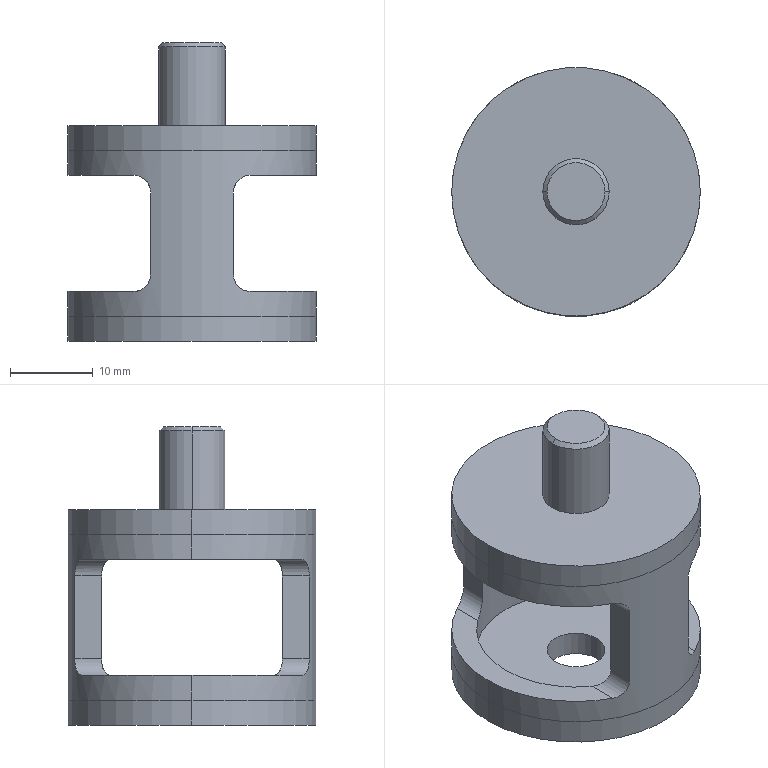Part | SolidWorks | features ICE 4, HoleWzd 2, Chamfer 1, Extrusion 1, Fillet 1 | 3 solids | 40 faces | box 30 x 30 x 36 mm | volume 6927 mm3 | cylinder 22 | plane 16 | cone 2 | commonest cylinder face diameters 4 x8 30 x6 6.8 x2 7 x2 8 x2 24 x2
STEP:
#1=CARTESIAN_POINT('',(-12.,0.,20.));
#2=VERTEX_POINT('',#1);
#3=CARTESIAN_POINT('',(12.,0.,20.));
#4=VERTEX_POINT('',#3);
#5=CARTESIAN_POINT('',(0.,0.,20.));
#6=DIRECTION('',(0.,0.,1.));
#7=DIRECTION('',(1.,0.,0.));
#8=AXIS2_PLACEMENT_3D('',#5,#6,#7);
#9=CIRCLE('',#8,12.);
#10=EDGE_CURVE('',#2,#4,#9,.T.);
#11=ORIENTED_EDGE('',*,*,#10,.T.);
#12=CARTESIAN_POINT('',(12.,0.,17.));
#13=VERTEX_POINT('',#12);
#14=CARTESIAN_POINT('',(12.,0.,20.));
#15=DIRECTION('',(0.,0.,-1.));
#16=VECTOR('',#15,1000.);
#17=LINE('',#14,#16);
#18=EDGE_CURVE('',#4,#13,#17,.T.);
#19=ORIENTED_EDGE('',*,*,#18,.T.);
#20=CARTESIAN_POINT('',(7.,-9.747,17.));
#21=VERTEX_POINT('',#20);
#22=CARTESIAN_POINT('',(0.,0.,17.));
#23=DIRECTION('',(0.,0.,1.));
#24=DIRECTION('',(1.,0.,0.));
#25=AXIS2_PLACEMENT_3D('',#22,#23,#24);
#26=CIRCLE('',#25,12.);
#27=EDGE_CURVE('',#21,#13,#26,.T.);
#28=ORIENTED_EDGE('',*,*,#27,.F.);
#29=CARTESIAN_POINT('',(5.,-10.909,15.));
#30=VERTEX_POINT('',#29);
#31=CARTESIAN_POINT('',(7.,-9.747,17.));
#32=CARTESIAN_POINT('',(6.768,-9.914,17.));
#33=CARTESIAN_POINT('',(6.535,-10.068,16.961));
#34=CARTESIAN_POINT('',(6.19,-10.281,16.833));
#35=CARTESIAN_POINT('',(6.076,-10.349,16.778));
#36=CARTESIAN_POINT('',(5.858,-10.474,16.647));
#37=CARTESIAN_POINT('',(5.753,-10.531,16.57));
#38=CARTESIAN_POINT('',(5.458,-10.689,16.302));
#39=CARTESIAN_POINT('',(5.294,-10.77,16.08));
#40=CARTESIAN_POINT('',(5.12,-10.853,15.696));
#41=CARTESIAN_POINT('',(5.076,-10.874,15.564));
#42=CARTESIAN_POINT('',(5.016,-10.902,15.288));
#43=CARTESIAN_POINT('',(5.,-10.909,15.144));
#44=CARTESIAN_POINT('',(5.,-10.909,15.));
#45=B_SPLINE_CURVE_WITH_KNOTS('',3,(#31,#32,#33,#34,#35,#36,#37,#38,#39,#40,#41,#42,#43,#44),.UNSPECIFIED.,.F.,.F.,(4,2,2,2,2,2,4),(0.,0.0008435,0.001265,0.001687,0.00253,0.002952,0.003374),.UNSPECIFIED.);
#46=EDGE_CURVE('',#21,#30,#45,.T.);
#47=ORIENTED_EDGE('',*,*,#46,.T.);
#48=CARTESIAN_POINT('',(5.,-10.909,5.));
#49=VERTEX_POINT('',#48);
#50=CARTESIAN_POINT('',(5.,-10.909,20.));
#51=DIRECTION('',(0.,0.,1.));
#52=VECTOR('',#51,1000.);
#53=LINE('',#50,#52);
#54=EDGE_CURVE('',#49,#30,#53,.T.);
#55=ORIENTED_EDGE('',*,*,#54,.F.);
#56=CARTESIAN_POINT('',(7.,-9.747,3.));
#57=VERTEX_POINT('',#56);
#58=CARTESIAN_POINT('',(5.,-10.909,5.));
#59=CARTESIAN_POINT('',(5.,-10.909,4.857));
#60=CARTESIAN_POINT('',(5.015,-10.902,4.716));
#61=CARTESIAN_POINT('',(5.075,-10.874,4.44));
#62=CARTESIAN_POINT('',(5.12,-10.853,4.305));
#63=CARTESIAN_POINT('',(5.291,-10.771,3.925));
#64=CARTESIAN_POINT('',(5.458,-10.689,3.7));
#65=CARTESIAN_POINT('',(5.75,-10.533,3.433));
#66=CARTESIAN_POINT('',(5.856,-10.475,3.355));
#67=CARTESIAN_POINT('',(6.074,-10.35,3.223));
#68=CARTESIAN_POINT('',(6.186,-10.283,3.169));
#69=CARTESIAN_POINT('',(6.534,-10.069,3.039));
#70=CARTESIAN_POINT('',(6.768,-9.913,3.));
#71=CARTESIAN_POINT('',(7.,-9.747,3.));
#72=B_SPLINE_CURVE_WITH_KNOTS('',3,(#58,#59,#60,#61,#62,#63,#64,#65,#66,#67,#68,#69,#70,#71),.UNSPECIFIED.,.F.,.F.,(4,2,2,2,2,2,4),(0.,0.000424,0.000848,0.001696,0.00212,0.002544,0.003392),.UNSPECIFIED.);
#73=EDGE_CURVE('',#49,#57,#72,.T.);
#74=ORIENTED_EDGE('',*,*,#73,.T.);
#75=CARTESIAN_POINT('',(12.,0.,3.));
#76=VERTEX_POINT('',#75);
#77=CARTESIAN_POINT('',(0.,0.,3.));
#78=DIRECTION('',(0.,0.,-1.));
#79=DIRECTION('',(-1.,0.,0.));
#80=AXIS2_PLACEMENT_3D('',#77,#78,#79);
#81=CIRCLE('',#80,12.);
#82=EDGE_CURVE('',#76,#57,#81,.T.);
#83=ORIENTED_EDGE('',*,*,#82,.F.);
#84=CARTESIAN_POINT('',(12.,0.,0.));
#85=VERTEX_POINT('',#84);
#86=CARTESIAN_POINT('',(12.,0.,20.));
#87=DIRECTION('',(0.,0.,-1.));
#88=VECTOR('',#87,1000.);
#89=LINE('',#86,#88);
#90=EDGE_CURVE('',#76,#85,#89,.T.);
#91=ORIENTED_EDGE('',*,*,#90,.T.);
#92=CARTESIAN_POINT('',(-12.,0.,0.));
#93=VERTEX_POINT('',#92);
#94=CARTESIAN_POINT('',(0.,0.,0.));
#95=DIRECTION('',(0.,0.,1.));
#96=DIRECTION('',(1.,0.,0.));
#97=AXIS2_PLACEMENT_3D('',#94,#95,#96);
#98=CIRCLE('',#97,12.);
#99=EDGE_CURVE('',#93,#85,#98,.T.);
#100=ORIENTED_EDGE('',*,*,#99,.F.);
#101=CARTESIAN_POINT('',(-12.,0.,3.));
#102=VERTEX_POINT('',#101);
#103=CARTESIAN_POINT('',(-12.,0.,20.));
#104=DIRECTION('',(0.,0.,-1.));
#105=VECTOR('',#104,1000.);
#106=LINE('',#103,#105);
#107=EDGE_CURVE('',#102,#93,#106,.T.);
#108=ORIENTED_EDGE('',*,*,#107,.F.);
#109=CARTESIAN_POINT('',(-7.,-9.747,3.));
#110=VERTEX_POINT('',#109);
#111=CARTESIAN_POINT('',(0.,0.,3.));
#112=DIRECTION('',(0.,0.,-1.));
#113=DIRECTION('',(-1.,0.,0.));
#114=AXIS2_PLACEMENT_3D('',#111,#112,#113);
#115=CIRCLE('',#114,12.);
#116=EDGE_CURVE('',#110,#102,#115,.T.);
#117=ORIENTED_EDGE('',*,*,#116,.F.);
#118=CARTESIAN_POINT('',(-5.,-10.909,5.));
#119=VERTEX_POINT('',#118);
#120=CARTESIAN_POINT('',(-7.,-9.747,3.));
#121=CARTESIAN_POINT('',(-6.768,-9.914,3.));
#122=CARTESIAN_POINT('',(-6.535,-10.068,3.039));
#123=CARTESIAN_POINT('',(-6.19,-10.281,3.167));
#124=CARTESIAN_POINT('',(-6.076,-10.349,3.222));
#125=CARTESIAN_POINT('',(-5.858,-10.474,3.353));
#126=CARTESIAN_POINT('',(-5.753,-10.531,3.43));
#127=CARTESIAN_POINT('',(-5.458,-10.689,3.698));
#128=CARTESIAN_POINT('',(-5.294,-10.77,3.92));
#129=CARTESIAN_POINT('',(-5.12,-10.853,4.304));
#130=CARTESIAN_POINT('',(-5.076,-10.874,4.436));
#131=CARTESIAN_POINT('',(-5.016,-10.902,4.712));
#132=CARTESIAN_POINT('',(-5.,-10.909,4.856));
#133=CARTESIAN_POINT('',(-5.,-10.909,5.));
#134=B_SPLINE_CURVE_WITH_KNOTS('',3,(#120,#121,#122,#123,#124,#125,#126,#127,#128,#129,#130,#131,#132,#133),.UNSPECIFIED.,.F.,.F.,(4,2,2,2,2,2,4),(0.,0.0008435,0.001265,0.001687,0.00253,0.002952,0.003374),.UNSPECIFIED.);
#135=EDGE_CURVE('',#110,#119,#134,.T.);
#136=ORIENTED_EDGE('',*,*,#135,.T.);
#137=CARTESIAN_POINT('',(-5.,-10.909,15.));
#138=VERTEX_POINT('',#137);
#139=CARTESIAN_POINT('',(-5.,-10.909,20.));
#140=DIRECTION('',(0.,0.,-1.));
#141=VECTOR('',#140,1000.);
#142=LINE('',#139,#141);
#143=EDGE_CURVE('',#138,#119,#142,.T.);
#144=ORIENTED_EDGE('',*,*,#143,.F.);
#145=CARTESIAN_POINT('',(-7.,-9.747,17.));
#146=VERTEX_POINT('',#145);
#147=CARTESIAN_POINT('',(-5.,-10.909,15.));
#148=CARTESIAN_POINT('',(-5.,-10.909,15.143));
#149=CARTESIAN_POINT('',(-5.015,-10.902,15.284));
#150=CARTESIAN_POINT('',(-5.075,-10.874,15.56));
#151=CARTESIAN_POINT('',(-5.12,-10.853,15.695));
#152=CARTESIAN_POINT('',(-5.291,-10.771,16.075));
#153=CARTESIAN_POINT('',(-5.458,-10.689,16.3));
#154=CARTESIAN_POINT('',(-5.75,-10.533,16.567));
#155=CARTESIAN_POINT('',(-5.856,-10.475,16.645));
#156=CARTESIAN_POINT('',(-6.074,-10.35,16.777));
#157=CARTESIAN_POINT('',(-6.186,-10.283,16.831));
#158=CARTESIAN_POINT('',(-6.534,-10.069,16.961));
#159=CARTESIAN_POINT('',(-6.768,-9.913,17.));
#160=CARTESIAN_POINT('',(-7.,-9.747,17.));
#161=B_SPLINE_CURVE_WITH_KNOTS('',3,(#147,#148,#149,#150,#151,#152,#153,#154,#155,#156,#157,#158,#159,#160),.UNSPECIFIED.,.F.,.F.,(4,2,2,2,2,2,4),(0.,0.000424,0.000848,0.001696,0.00212,0.002544,0.003392),.UNSPECIFIED.);
#162=EDGE_CURVE('',#138,#146,#161,.T.);
#163=ORIENTED_EDGE('',*,*,#162,.T.);
#164=CARTESIAN_POINT('',(-12.,0.,17.));
#165=VERTEX_POINT('',#164);
#166=CARTESIAN_POINT('',(0.,0.,17.));
#167=DIRECTION('',(0.,0.,1.));
#168=DIRECTION('',(1.,0.,0.));
#169=AXIS2_PLACEMENT_3D('',#166,#167,#168);
#170=CIRCLE('',#169,12.);
#171=EDGE_CURVE('',#165,#146,#170,.T.);
#172=ORIENTED_EDGE('',*,*,#171,.F.);
#173=CARTESIAN_POINT('',(-12.,0.,20.));
#174=DIRECTION('',(0.,0.,-1.));
#175=VECTOR('',#174,1000.);
#176=LINE('',#173,#175);
#177=EDGE_CURVE('',#2,#165,#176,.T.);
#178=ORIENTED_EDGE('',*,*,#177,.F.);
#179=EDGE_LOOP('',(#11,#19,#28,#47,#55,#74,#83,#91,#100,#108,#117,#136,#144,#163,#172,#178));
#180=FACE_OUTER_BOUND('',#179,.T.);
#181=CARTESIAN_POINT('',(0.,0.,20.));
#182=DIRECTION('',(0.,0.,-1.));
#183=DIRECTION('',(-1.,0.,0.));
#184=AXIS2_PLACEMENT_3D('',#181,#182,#183);
#185=CYLINDRICAL_SURFACE('',#184,12.);
#186=ADVANCED_FACE('',(#180),#185,.F.);
#187=CARTESIAN_POINT('',(15.,0.,20.));
#188=VERTEX_POINT('',#187);
#189=CARTESIAN_POINT('',(-15.,0.,20.));
#190=VERTEX_POINT('',#189);
#191=CARTESIAN_POINT('',(0.,0.,20.));
#192=DIRECTION('',(0.,0.,1.));
#193=DIRECTION('',(1.,0.,0.));
#194=AXIS2_PLACEMENT_3D('',#191,#192,#193);
#195=CIRCLE('',#194,15.);
#196=EDGE_CURVE('',#188,#190,#195,.T.);
#197=ORIENTED_EDGE('',*,*,#196,.F.);
#198=CARTESIAN_POINT('',(15.,0.,17.));
#199=VERTEX_POINT('',#198);
#200=CARTESIAN_POINT('',(15.,0.,20.));
#201=DIRECTION('',(0.,0.,-1.));
#202=VECTOR('',#201,1000.);
#203=LINE('',#200,#202);
#204=EDGE_CURVE('',#188,#199,#203,.T.);
#205=ORIENTED_EDGE('',*,*,#204,.T.);
#206=CARTESIAN_POINT('',(7.,13.266,17.));
#207=VERTEX_POINT('',#206);
#208=CARTESIAN_POINT('',(0.,0.,17.));
#209=DIRECTION('',(0.,0.,1.));
#210=DIRECTION('',(1.,0.,0.));
#211=AXIS2_PLACEMENT_3D('',#208,#209,#210);
#212=CIRCLE('',#211,15.);
#213=EDGE_CURVE('',#199,#207,#212,.T.);
#214=ORIENTED_EDGE('',*,*,#213,.T.);
#215=CARTESIAN_POINT('',(5.,14.142,15.));
#216=VERTEX_POINT('',#215);
#217=CARTESIAN_POINT('',(7.,13.266,17.));
#218=CARTESIAN_POINT('',(6.755,13.396,17.));
#219=CARTESIAN_POINT('',(6.512,13.515,16.956));
#220=CARTESIAN_POINT('',(6.038,13.733,16.772));
#221=CARTESIAN_POINT('',(5.819,13.827,16.636));
#222=CARTESIAN_POINT('',(5.53,13.944,16.362));
#223=CARTESIAN_POINT('',(5.443,13.978,16.262));
#224=CARTESIAN_POINT('',(5.289,14.037,16.045));
#225=CARTESIAN_POINT('',(5.222,14.062,15.925));
#226=CARTESIAN_POINT('',(5.113,14.102,15.676));
#227=CARTESIAN_POINT('',(5.071,14.117,15.546));
#228=CARTESIAN_POINT('',(5.015,14.137,15.278));
#229=CARTESIAN_POINT('',(5.,14.142,15.139));
#230=CARTESIAN_POINT('',(5.,14.142,15.));
#231=B_SPLINE_CURVE_WITH_KNOTS('',3,(#217,#218,#219,#220,#221,#222,#223,#224,#225,#226,#227,#228,#229,#230),.UNSPECIFIED.,.F.,.F.,(4,2,2,2,2,2,4),(0.,0.0008196,0.001639,0.002049,0.002459,0.002869,0.003279),.UNSPECIFIED.);
#232=EDGE_CURVE('',#207,#216,#231,.T.);
#233=ORIENTED_EDGE('',*,*,#232,.T.);
#234=CARTESIAN_POINT('',(5.,14.142,5.));
#235=VERTEX_POINT('',#234);
#236=CARTESIAN_POINT('',(5.,14.142,20.));
#237=DIRECTION('',(0.,0.,-1.));
#238=VECTOR('',#237,1000.);
#239=LINE('',#236,#238);
#240=EDGE_CURVE('',#216,#235,#239,.T.);
#241=ORIENTED_EDGE('',*,*,#240,.T.);
#242=CARTESIAN_POINT('',(7.,13.266,3.));
#243=VERTEX_POINT('',#242);
#244=CARTESIAN_POINT('',(5.,14.142,5.));
#245=CARTESIAN_POINT('',(5.,14.142,4.861));
#246=CARTESIAN_POINT('',(5.014,14.137,4.725));
#247=CARTESIAN_POINT('',(5.07,14.117,4.458));
#248=CARTESIAN_POINT('',(5.112,14.102,4.326));
#249=CARTESIAN_POINT('',(5.275,14.043,3.953));
#250=CARTESIAN_POINT('',(5.434,13.983,3.729));
#251=CARTESIAN_POINT('',(5.72,13.867,3.458));
#252=CARTESIAN_POINT('',(5.824,13.824,3.377));
#253=CARTESIAN_POINT('',(6.043,13.729,3.239));
#254=CARTESIAN_POINT('',(6.156,13.679,3.182));
#255=CARTESIAN_POINT('',(6.392,13.571,3.091));
#256=CARTESIAN_POINT('',(6.513,13.513,3.056));
#257=CARTESIAN_POINT('',(6.756,13.393,3.011));
#258=CARTESIAN_POINT('',(6.878,13.331,3.));
#259=CARTESIAN_POINT('',(7.,13.266,3.));
#260=B_SPLINE_CURVE_WITH_KNOTS('',3,(#244,#245,#246,#247,#248,#249,#250,#251,#252,#253,#254,#255,#256,#257,#258,#259),.UNSPECIFIED.,.F.,.F.,(4,2,2,2,2,2,2,4),(0.,0.0004099,0.0008198,0.00164,0.002049,0.002459,0.002869,0.003279),.UNSPECIFIED.);
#261=EDGE_CURVE('',#235,#243,#260,.T.);
#262=ORIENTED_EDGE('',*,*,#261,.T.);
#263=CARTESIAN_POINT('',(15.,0.,3.));
#264=VERTEX_POINT('',#263);
#265=CARTESIAN_POINT('',(0.,0.,3.));
#266=DIRECTION('',(0.,0.,-1.));
#267=DIRECTION('',(-1.,0.,0.));
#268=AXIS2_PLACEMENT_3D('',#265,#266,#267);
#269=CIRCLE('',#268,15.);
#270=EDGE_CURVE('',#243,#264,#269,.T.);
#271=ORIENTED_EDGE('',*,*,#270,.T.);
#272=CARTESIAN_POINT('',(15.,0.,0.));
#273=VERTEX_POINT('',#272);
#274=CARTESIAN_POINT('',(15.,0.,20.));
#275=DIRECTION('',(0.,0.,-1.));
#276=VECTOR('',#275,1000.);
#277=LINE('',#274,#276);
#278=EDGE_CURVE('',#264,#273,#277,.T.);
#279=ORIENTED_EDGE('',*,*,#278,.T.);
#280=CARTESIAN_POINT('',(-15.,0.,0.));
#281=VERTEX_POINT('',#280);
#282=CARTESIAN_POINT('',(0.,0.,0.));
#283=DIRECTION('',(0.,0.,1.));
#284=DIRECTION('',(1.,0.,0.));
#285=AXIS2_PLACEMENT_3D('',#282,#283,#284);
#286=CIRCLE('',#285,15.);
#287=EDGE_CURVE('',#273,#281,#286,.T.);
#288=ORIENTED_EDGE('',*,*,#287,.T.);
#289=CARTESIAN_POINT('',(-15.,0.,3.));
#290=VERTEX_POINT('',#289);
#291=CARTESIAN_POINT('',(-15.,0.,20.));
#292=DIRECTION('',(0.,0.,-1.));
#293=VECTOR('',#292,1000.);
#294=LINE('',#291,#293);
#295=EDGE_CURVE('',#290,#281,#294,.T.);
#296=ORIENTED_EDGE('',*,*,#295,.F.);
#297=CARTESIAN_POINT('',(-7.,13.266,3.));
#298=VERTEX_POINT('',#297);
#299=CARTESIAN_POINT('',(0.,0.,3.));
#300=DIRECTION('',(0.,0.,-1.));
#301=DIRECTION('',(-1.,0.,0.));
#302=AXIS2_PLACEMENT_3D('',#299,#300,#301);
#303=CIRCLE('',#302,15.);
#304=EDGE_CURVE('',#290,#298,#303,.T.);
#305=ORIENTED_EDGE('',*,*,#304,.T.);
#306=CARTESIAN_POINT('',(-5.,14.142,5.));
#307=VERTEX_POINT('',#306);
#308=CARTESIAN_POINT('',(-7.,13.266,3.));
#309=CARTESIAN_POINT('',(-6.755,13.396,3.));
#310=CARTESIAN_POINT('',(-6.512,13.515,3.044));
#311=CARTESIAN_POINT('',(-6.038,13.733,3.228));
#312=CARTESIAN_POINT('',(-5.819,13.827,3.364));
#313=CARTESIAN_POINT('',(-5.53,13.944,3.638));
#314=CARTESIAN_POINT('',(-5.443,13.978,3.738));
#315=CARTESIAN_POINT('',(-5.289,14.037,3.955));
#316=CARTESIAN_POINT('',(-5.222,14.062,4.075));
#317=CARTESIAN_POINT('',(-5.113,14.102,4.324));
#318=CARTESIAN_POINT('',(-5.071,14.117,4.454));
#319=CARTESIAN_POINT('',(-5.015,14.137,4.722));
#320=CARTESIAN_POINT('',(-5.,14.142,4.861));
#321=CARTESIAN_POINT('',(-5.,14.142,5.));
#322=B_SPLINE_CURVE_WITH_KNOTS('',3,(#308,#309,#310,#311,#312,#313,#314,#315,#316,#317,#318,#319,#320,#321),.UNSPECIFIED.,.F.,.F.,(4,2,2,2,2,2,4),(0.,0.0008196,0.001639,0.002049,0.002459,0.002869,0.003279),.UNSPECIFIED.);
#323=EDGE_CURVE('',#298,#307,#322,.T.);
#324=ORIENTED_EDGE('',*,*,#323,.T.);
#325=CARTESIAN_POINT('',(-5.,14.142,15.));
#326=VERTEX_POINT('',#325);
#327=CARTESIAN_POINT('',(-5.,14.142,20.));
#328=DIRECTION('',(0.,0.,1.));
#329=VECTOR('',#328,1000.);
#330=LINE('',#327,#329);
#331=EDGE_CURVE('',#307,#326,#330,.T.);
#332=ORIENTED_EDGE('',*,*,#331,.T.);
#333=CARTESIAN_POINT('',(-7.,13.266,17.));
#334=VERTEX_POINT('',#333);
#335=CARTESIAN_POINT('',(-5.,14.142,15.));
#336=CARTESIAN_POINT('',(-5.,14.142,15.139));
#337=CARTESIAN_POINT('',(-5.014,14.137,15.275));
#338=CARTESIAN_POINT('',(-5.07,14.117,15.542));
#339=CARTESIAN_POINT('',(-5.112,14.102,15.674));
#340=CARTESIAN_POINT('',(-5.275,14.043,16.047));
#341=CARTESIAN_POINT('',(-5.434,13.983,16.271));
#342=CARTESIAN_POINT('',(-5.72,13.867,16.542));
#343=CARTESIAN_POINT('',(-5.824,13.824,16.623));
#344=CARTESIAN_POINT('',(-6.043,13.729,16.761));
#345=CARTESIAN_POINT('',(-6.156,13.679,16.818));
#346=CARTESIAN_POINT('',(-6.392,13.571,16.909));
#347=CARTESIAN_POINT('',(-6.513,13.513,16.944));
#348=CARTESIAN_POINT('',(-6.756,13.393,16.989));
#349=CARTESIAN_POINT('',(-6.878,13.331,17.));
#350=CARTESIAN_POINT('',(-7.,13.266,17.));
#351=B_SPLINE_CURVE_WITH_KNOTS('',3,(#335,#336,#337,#338,#339,#340,#341,#342,#343,#344,#345,#346,#347,#348,#349,#350),.UNSPECIFIED.,.F.,.F.,(4,2,2,2,2,2,2,4),(0.,0.0004099,0.0008198,0.00164,0.002049,0.002459,0.002869,0.003279),.UNSPECIFIED.);
#352=EDGE_CURVE('',#326,#334,#351,.T.);
#353=ORIENTED_EDGE('',*,*,#352,.T.);
#354=CARTESIAN_POINT('',(-15.,0.,17.));
#355=VERTEX_POINT('',#354);
#356=CARTESIAN_POINT('',(0.,0.,17.));
#357=DIRECTION('',(0.,0.,1.));
#358=DIRECTION('',(1.,0.,0.));
#359=AXIS2_PLACEMENT_3D('',#356,#357,#358);
#360=CIRCLE('',#359,15.);
#361=EDGE_CURVE('',#334,#355,#360,.T.);
#362=ORIENTED_EDGE('',*,*,#361,.T.);
#363=CARTESIAN_POINT('',(-15.,0.,20.));
#364=DIRECTION('',(0.,0.,-1.));
#365=VECTOR('',#364,1000.);
#366=LINE('',#363,#365);
#367=EDGE_CURVE('',#190,#355,#366,.T.);
#368=ORIENTED_EDGE('',*,*,#367,.F.);
#369=EDGE_LOOP('',(#197,#205,#214,#233,#241,#262,#271,#279,#288,#296,#305,#324,#332,#353,#362,#368));
#370=FACE_OUTER_BOUND('',#369,.T.);
#371=CARTESIAN_POINT('',(0.,0.,20.));
#372=DIRECTION('',(0.,0.,-1.));
#373=DIRECTION('',(-1.,0.,0.));
#374=AXIS2_PLACEMENT_3D('',#371,#372,#373);
#375=CYLINDRICAL_SURFACE('',#374,15.);
#376=ADVANCED_FACE('',(#370),#375,.T.);
#377=CARTESIAN_POINT('',(0.,0.,20.));
#378=DIRECTION('',(0.,0.,1.));
#379=DIRECTION('',(1.,0.,0.));
#380=AXIS2_PLACEMENT_3D('',#377,#378,#379);
#381=CIRCLE('',#380,15.);
#382=EDGE_CURVE('',#190,#188,#381,.T.);
#383=ORIENTED_EDGE('',*,*,#382,.T.);
#384=ORIENTED_EDGE('',*,*,#196,.T.);
#385=EDGE_LOOP('',(#383,#384));
#386=FACE_OUTER_BOUND('',#385,.T.);
#387=ORIENTED_EDGE('',*,*,#10,.F.);
#388=CARTESIAN_POINT('',(0.,0.,20.));
#389=DIRECTION('',(0.,0.,1.));
#390=DIRECTION('',(1.,0.,0.));
#391=AXIS2_PLACEMENT_3D('',#388,#389,#390);
#392=CIRCLE('',#391,12.);
#393=EDGE_CURVE('',#4,#2,#392,.T.);
#394=ORIENTED_EDGE('',*,*,#393,.F.);
#395=EDGE_LOOP('',(#387,#394));
#396=FACE_BOUND('',#395,.T.);
#397=CARTESIAN_POINT('',(0.,0.,20.));
#398=DIRECTION('',(0.,0.,1.));
#399=DIRECTION('',(1.,0.,0.));
#400=AXIS2_PLACEMENT_3D('',#397,#398,#399);
#401=PLANE('',#400);
#402=ADVANCED_FACE('',(#386,#396),#401,.T.);
#403=CARTESIAN_POINT('',(0.,0.,0.));
#404=DIRECTION('',(0.,0.,1.));
#405=DIRECTION('',(1.,0.,0.));
#406=AXIS2_PLACEMENT_3D('',#403,#404,#405);
#407=CIRCLE('',#406,15.);
#408=EDGE_CURVE('',#281,#273,#407,.T.);
#409=ORIENTED_EDGE('',*,*,#408,.F.);
#410=ORIENTED_EDGE('',*,*,#287,.F.);
#411=EDGE_LOOP('',(#409,#410));
#412=FACE_OUTER_BOUND('',#411,.T.);
#413=ORIENTED_EDGE('',*,*,#99,.T.);
#414=CARTESIAN_POINT('',(0.,0.,0.));
#415=DIRECTION('',(0.,0.,1.));
#416=DIRECTION('',(1.,0.,0.));
#417=AXIS2_PLACEMENT_3D('',#414,#415,#416);
#418=CIRCLE('',#417,12.);
#419=EDGE_CURVE('',#85,#93,#418,.T.);
#420=ORIENTED_EDGE('',*,*,#419,.T.);
#421=EDGE_LOOP('',(#413,#420));
#422=FACE_BOUND('',#421,.T.);
#423=CARTESIAN_POINT('',(0.,0.,0.));
#424=DIRECTION('',(0.,0.,1.));
#425=DIRECTION('',(1.,0.,0.));
#426=AXIS2_PLACEMENT_3D('',#423,#424,#425);
#427=PLANE('',#426);
#428=ADVANCED_FACE('',(#412,#422),#427,.F.);
#429=ORIENTED_EDGE('',*,*,#204,.F.);
#430=ORIENTED_EDGE('',*,*,#382,.F.);
#431=ORIENTED_EDGE('',*,*,#367,.T.);
#432=CARTESIAN_POINT('',(-7.,-13.266,17.));
#433=VERTEX_POINT('',#432);
#434=CARTESIAN_POINT('',(0.,0.,17.));
#435=DIRECTION('',(0.,0.,1.));
#436=DIRECTION('',(1.,0.,0.));
#437=AXIS2_PLACEMENT_3D('',#434,#435,#436);
#438=CIRCLE('',#437,15.);
#439=EDGE_CURVE('',#355,#433,#438,.T.);
#440=ORIENTED_EDGE('',*,*,#439,.T.);
#441=CARTESIAN_POINT('',(-5.,-14.142,15.));
#442=VERTEX_POINT('',#441);
#443=CARTESIAN_POINT('',(-7.,-13.266,17.));
#444=CARTESIAN_POINT('',(-6.755,-13.396,17.));
#445=CARTESIAN_POINT('',(-6.512,-13.515,16.956));
#446=CARTESIAN_POINT('',(-6.038,-13.733,16.772));
#447=CARTESIAN_POINT('',(-5.819,-13.827,16.636));
#448=CARTESIAN_POINT('',(-5.53,-13.944,16.362));
#449=CARTESIAN_POINT('',(-5.443,-13.978,16.262));
#450=CARTESIAN_POINT('',(-5.289,-14.037,16.045));
#451=CARTESIAN_POINT('',(-5.222,-14.062,15.925));
#452=CARTESIAN_POINT('',(-5.113,-14.102,15.676));
#453=CARTESIAN_POINT('',(-5.071,-14.117,15.546));
#454=CARTESIAN_POINT('',(-5.015,-14.137,15.278));
#455=CARTESIAN_POINT('',(-5.,-14.142,15.139));
#456=CARTESIAN_POINT('',(-5.,-14.142,15.));
#457=B_SPLINE_CURVE_WITH_KNOTS('',3,(#443,#444,#445,#446,#447,#448,#449,#450,#451,#452,#453,#454,#455,#456),.UNSPECIFIED.,.F.,.F.,(4,2,2,2,2,2,4),(0.,0.0008196,0.001639,0.002049,0.002459,0.002869,0.003279),.UNSPECIFIED.);
#458=EDGE_CURVE('',#433,#442,#457,.T.);
#459=ORIENTED_EDGE('',*,*,#458,.T.);
#460=CARTESIAN_POINT('',(-5.,-14.142,5.));
#461=VERTEX_POINT('',#460);
#462=CARTESIAN_POINT('',(-5.,-14.142,20.));
#463=DIRECTION('',(0.,0.,-1.));
#464=VECTOR('',#463,1000.);
#465=LINE('',#462,#464);
#466=EDGE_CURVE('',#442,#461,#465,.T.);
#467=ORIENTED_EDGE('',*,*,#466,.T.);
#468=CARTESIAN_POINT('',(-7.,-13.266,3.));
#469=VERTEX_POINT('',#468);
#470=CARTESIAN_POINT('',(-5.,-14.142,5.));
#471=CARTESIAN_POINT('',(-5.,-14.142,4.861));
#472=CARTESIAN_POINT('',(-5.014,-14.137,4.725));
#473=CARTESIAN_POINT('',(-5.07,-14.117,4.458));
#474=CARTESIAN_POINT('',(-5.112,-14.102,4.326));
#475=CARTESIAN_POINT('',(-5.275,-14.043,3.953));
#476=CARTESIAN_POINT('',(-5.434,-13.983,3.729));
#477=CARTESIAN_POINT('',(-5.72,-13.867,3.458));
#478=CARTESIAN_POINT('',(-5.824,-13.824,3.377));
#479=CARTESIAN_POINT('',(-6.043,-13.729,3.239));
#480=CARTESIAN_POINT('',(-6.156,-13.679,3.182));
#481=CARTESIAN_POINT('',(-6.392,-13.571,3.091));
#482=CARTESIAN_POINT('',(-6.513,-13.513,3.056));
#483=CARTESIAN_POINT('',(-6.756,-13.393,3.011));
#484=CARTESIAN_POINT('',(-6.878,-13.331,3.));
#485=CARTESIAN_POINT('',(-7.,-13.266,3.));
#486=B_SPLINE_CURVE_WITH_KNOTS('',3,(#470,#471,#472,#473,#474,#475,#476,#477,#478,#479,#480,#481,#482,#483,#484,#485),.UNSPECIFIED.,.F.,.F.,(4,2,2,2,2,2,2,4),(0.,0.0004099,0.0008198,0.00164,0.002049,0.002459,0.002869,0.003279),.UNSPECIFIED.);
#487=EDGE_CURVE('',#461,#469,#486,.T.);
#488=ORIENTED_EDGE('',*,*,#487,.T.);
#489=CARTESIAN_POINT('',(0.,0.,3.));
#490=DIRECTION('',(0.,0.,-1.));
#491=DIRECTION('',(-1.,0.,0.));
#492=AXIS2_PLACEMENT_3D('',#489,#490,#491);
#493=CIRCLE('',#492,15.);
#494=EDGE_CURVE('',#469,#290,#493,.T.);
#495=ORIENTED_EDGE('',*,*,#494,.T.);
#496=ORIENTED_EDGE('',*,*,#295,.T.);
#497=ORIENTED_EDGE('',*,*,#408,.T.);
#498=ORIENTED_EDGE('',*,*,#278,.F.);
#499=CARTESIAN_POINT('',(7.,-13.266,3.));
#500=VERTEX_POINT('',#499);
#501=CARTESIAN_POINT('',(0.,0.,3.));
#502=DIRECTION('',(0.,0.,-1.));
#503=DIRECTION('',(-1.,0.,0.));
#504=AXIS2_PLACEMENT_3D('',#501,#502,#503);
#505=CIRCLE('',#504,15.);
#506=EDGE_CURVE('',#264,#500,#505,.T.);
#507=ORIENTED_EDGE('',*,*,#506,.T.);
#508=CARTESIAN_POINT('',(5.,-14.142,5.));
#509=VERTEX_POINT('',#508);
#510=CARTESIAN_POINT('',(7.,-13.266,3.));
#511=CARTESIAN_POINT('',(6.755,-13.396,3.));
#512=CARTESIAN_POINT('',(6.512,-13.515,3.044));
#513=CARTESIAN_POINT('',(6.038,-13.733,3.228));
#514=CARTESIAN_POINT('',(5.819,-13.827,3.364));
#515=CARTESIAN_POINT('',(5.53,-13.944,3.638));
#516=CARTESIAN_POINT('',(5.443,-13.978,3.738));
#517=CARTESIAN_POINT('',(5.289,-14.037,3.955));
#518=CARTESIAN_POINT('',(5.222,-14.062,4.075));
#519=CARTESIAN_POINT('',(5.113,-14.102,4.324));
#520=CARTESIAN_POINT('',(5.071,-14.117,4.454));
#521=CARTESIAN_POINT('',(5.015,-14.137,4.722));
#522=CARTESIAN_POINT('',(5.,-14.142,4.861));
#523=CARTESIAN_POINT('',(5.,-14.142,5.));
#524=B_SPLINE_CURVE_WITH_KNOTS('',3,(#510,#511,#512,#513,#514,#515,#516,#517,#518,#519,#520,#521,#522,#523),.UNSPECIFIED.,.F.,.F.,(4,2,2,2,2,2,4),(0.,0.0008196,0.001639,0.002049,0.002459,0.002869,0.003279),.UNSPECIFIED.);
#525=EDGE_CURVE('',#500,#509,#524,.T.);
#526=ORIENTED_EDGE('',*,*,#525,.T.);
#527=CARTESIAN_POINT('',(5.,-14.142,15.));
#528=VERTEX_POINT('',#527);
#529=CARTESIAN_POINT('',(5.,-14.142,20.));
#530=DIRECTION('',(0.,0.,1.));
#531=VECTOR('',#530,1000.);
#532=LINE('',#529,#531);
#533=EDGE_CURVE('',#509,#528,#532,.T.);
#534=ORIENTED_EDGE('',*,*,#533,.T.);
#535=CARTESIAN_POINT('',(7.,-13.266,17.));
#536=VERTEX_POINT('',#535);
#537=CARTESIAN_POINT('',(5.,-14.142,15.));
#538=CARTESIAN_POINT('',(5.,-14.142,15.139));
#539=CARTESIAN_POINT('',(5.014,-14.137,15.275));
#540=CARTESIAN_POINT('',(5.07,-14.117,15.542));
#541=CARTESIAN_POINT('',(5.112,-14.102,15.674));
#542=CARTESIAN_POINT('',(5.275,-14.043,16.047));
#543=CARTESIAN_POINT('',(5.434,-13.983,16.271));
#544=CARTESIAN_POINT('',(5.72,-13.867,16.542));
#545=CARTESIAN_POINT('',(5.824,-13.824,16.623));
#546=CARTESIAN_POINT('',(6.043,-13.729,16.761));
#547=CARTESIAN_POINT('',(6.156,-13.679,16.818));
#548=CARTESIAN_POINT('',(6.392,-13.571,16.909));
#549=CARTESIAN_POINT('',(6.513,-13.513,16.944));
#550=CARTESIAN_POINT('',(6.756,-13.393,16.989));
#551=CARTESIAN_POINT('',(6.878,-13.331,17.));
#552=CARTESIAN_POINT('',(7.,-13.266,17.));
#553=B_SPLINE_CURVE_WITH_KNOTS('',3,(#537,#538,#539,#540,#541,#542,#543,#544,#545,#546,#547,#548,#549,#550,#551,#552),.UNSPECIFIED.,.F.,.F.,(4,2,2,2,2,2,2,4),(0.,0.0004099,0.0008198,0.00164,0.002049,0.002459,0.002869,0.003279),.UNSPECIFIED.);
#554=EDGE_CURVE('',#528,#536,#553,.T.);
#555=ORIENTED_EDGE('',*,*,#554,.T.);
#556=CARTESIAN_POINT('',(0.,0.,17.));
#557=DIRECTION('',(0.,0.,1.));
#558=DIRECTION('',(1.,0.,0.));
#559=AXIS2_PLACEMENT_3D('',#556,#557,#558);
#560=CIRCLE('',#559,15.);
#561=EDGE_CURVE('',#536,#199,#560,.T.);
#562=ORIENTED_EDGE('',*,*,#561,.T.);
#563=EDGE_LOOP('',(#429,#430,#431,#440,#459,#467,#488,#495,#496,#497,#498,#507,#526,#534,#555,#562));
#564=FACE_OUTER_BOUND('',#563,.T.);
#565=CARTESIAN_POINT('',(0.,0.,20.));
#566=DIRECTION('',(0.,0.,-1.));
#567=DIRECTION('',(-1.,0.,0.));
#568=AXIS2_PLACEMENT_3D('',#565,#566,#567);
#569=CYLINDRICAL_SURFACE('',#568,15.);
#570=ADVANCED_FACE('',(#564),#569,.T.);
#571=ORIENTED_EDGE('',*,*,#18,.F.);
#572=ORIENTED_EDGE('',*,*,#393,.T.);
#573=ORIENTED_EDGE('',*,*,#177,.T.);
#574=CARTESIAN_POINT('',(-7.,9.747,17.));
#575=VERTEX_POINT('',#574);
#576=CARTESIAN_POINT('',(0.,0.,17.));
#577=DIRECTION('',(0.,0.,1.));
#578=DIRECTION('',(1.,0.,0.));
#579=AXIS2_PLACEMENT_3D('',#576,#577,#578);
#580=CIRCLE('',#579,12.);
#581=EDGE_CURVE('',#575,#165,#580,.T.);
#582=ORIENTED_EDGE('',*,*,#581,.F.);
#583=CARTESIAN_POINT('',(-5.,10.909,15.));
#584=VERTEX_POINT('',#583);
#585=CARTESIAN_POINT('',(-7.,9.747,17.));
#586=CARTESIAN_POINT('',(-6.768,9.914,17.));
#587=CARTESIAN_POINT('',(-6.535,10.068,16.961));
#588=CARTESIAN_POINT('',(-6.19,10.281,16.833));
#589=CARTESIAN_POINT('',(-6.076,10.349,16.778));
#590=CARTESIAN_POINT('',(-5.858,10.474,16.647));
#591=CARTESIAN_POINT('',(-5.753,10.531,16.57));
#592=CARTESIAN_POINT('',(-5.458,10.689,16.302));
#593=CARTESIAN_POINT('',(-5.294,10.77,16.08));
#594=CARTESIAN_POINT('',(-5.12,10.853,15.696));
#595=CARTESIAN_POINT('',(-5.076,10.874,15.564));
#596=CARTESIAN_POINT('',(-5.016,10.902,15.288));
#597=CARTESIAN_POINT('',(-5.,10.909,15.144));
#598=CARTESIAN_POINT('',(-5.,10.909,15.));
#599=B_SPLINE_CURVE_WITH_KNOTS('',3,(#585,#586,#587,#588,#589,#590,#591,#592,#593,#594,#595,#596,#597,#598),.UNSPECIFIED.,.F.,.F.,(4,2,2,2,2,2,4),(0.,0.0008435,0.001265,0.001687,0.00253,0.002952,0.003374),.UNSPECIFIED.);
#600=EDGE_CURVE('',#575,#584,#599,.T.);
#601=ORIENTED_EDGE('',*,*,#600,.T.);
#602=CARTESIAN_POINT('',(-5.,10.909,5.));
#603=VERTEX_POINT('',#602);
#604=CARTESIAN_POINT('',(-5.,10.909,20.));
#605=DIRECTION('',(0.,0.,1.));
#606=VECTOR('',#605,1000.);
#607=LINE('',#604,#606);
#608=EDGE_CURVE('',#603,#584,#607,.T.);
#609=ORIENTED_EDGE('',*,*,#608,.F.);
#610=CARTESIAN_POINT('',(-7.,9.747,3.));
#611=VERTEX_POINT('',#610);
#612=CARTESIAN_POINT('',(-5.,10.909,5.));
#613=CARTESIAN_POINT('',(-5.,10.909,4.857));
#614=CARTESIAN_POINT('',(-5.015,10.902,4.716));
#615=CARTESIAN_POINT('',(-5.075,10.874,4.44));
#616=CARTESIAN_POINT('',(-5.12,10.853,4.305));
#617=CARTESIAN_POINT('',(-5.291,10.771,3.925));
#618=CARTESIAN_POINT('',(-5.458,10.689,3.7));
#619=CARTESIAN_POINT('',(-5.75,10.533,3.433));
#620=CARTESIAN_POINT('',(-5.856,10.475,3.355));
#621=CARTESIAN_POINT('',(-6.074,10.35,3.223));
#622=CARTESIAN_POINT('',(-6.186,10.283,3.169));
#623=CARTESIAN_POINT('',(-6.534,10.069,3.039));
#624=CARTESIAN_POINT('',(-6.768,9.913,3.));
#625=CARTESIAN_POINT('',(-7.,9.747,3.));
#626=B_SPLINE_CURVE_WITH_KNOTS('',3,(#612,#613,#614,#615,#616,#617,#618,#619,#620,#621,#622,#623,#624,#625),.UNSPECIFIED.,.F.,.F.,(4,2,2,2,2,2,4),(0.,0.000424,0.000848,0.001696,0.00212,0.002544,0.003392),.UNSPECIFIED.);
#627=EDGE_CURVE('',#603,#611,#626,.T.);
#628=ORIENTED_EDGE('',*,*,#627,.T.);
#629=CARTESIAN_POINT('',(0.,0.,3.));
#630=DIRECTION('',(0.,0.,-1.));
#631=DIRECTION('',(-1.,0.,0.));
#632=AXIS2_PLACEMENT_3D('',#629,#630,#631);
#633=CIRCLE('',#632,12.);
#634=EDGE_CURVE('',#102,#611,#633,.T.);
#635=ORIENTED_EDGE('',*,*,#634,.F.);
#636=ORIENTED_EDGE('',*,*,#107,.T.);
#637=ORIENTED_EDGE('',*,*,#419,.F.);
#638=ORIENTED_EDGE('',*,*,#90,.F.);
#639=CARTESIAN_POINT('',(7.,9.747,3.));
#640=VERTEX_POINT('',#639);
#641=CARTESIAN_POINT('',(0.,0.,3.));
#642=DIRECTION('',(0.,0.,-1.));
#643=DIRECTION('',(-1.,0.,0.));
#644=AXIS2_PLACEMENT_3D('',#641,#642,#643);
#645=CIRCLE('',#644,12.);
#646=EDGE_CURVE('',#640,#76,#645,.T.);
#647=ORIENTED_EDGE('',*,*,#646,.F.);
#648=CARTESIAN_POINT('',(5.,10.909,5.));
#649=VERTEX_POINT('',#648);
#650=CARTESIAN_POINT('',(7.,9.747,3.));
#651=CARTESIAN_POINT('',(6.768,9.914,3.));
#652=CARTESIAN_POINT('',(6.535,10.068,3.039));
#653=CARTESIAN_POINT('',(6.19,10.281,3.167));
#654=CARTESIAN_POINT('',(6.076,10.349,3.222));
#655=CARTESIAN_POINT('',(5.858,10.474,3.353));
#656=CARTESIAN_POINT('',(5.753,10.531,3.43));
#657=CARTESIAN_POINT('',(5.458,10.689,3.698));
#658=CARTESIAN_POINT('',(5.294,10.77,3.92));
#659=CARTESIAN_POINT('',(5.12,10.853,4.304));
#660=CARTESIAN_POINT('',(5.076,10.874,4.436));
#661=CARTESIAN_POINT('',(5.016,10.902,4.712));
#662=CARTESIAN_POINT('',(5.,10.909,4.856));
#663=CARTESIAN_POINT('',(5.,10.909,5.));
#664=B_SPLINE_CURVE_WITH_KNOTS('',3,(#650,#651,#652,#653,#654,#655,#656,#657,#658,#659,#660,#661,#662,#663),.UNSPECIFIED.,.F.,.F.,(4,2,2,2,2,2,4),(0.,0.0008435,0.001265,0.001687,0.00253,0.002952,0.003374),.UNSPECIFIED.);
#665=EDGE_CURVE('',#640,#649,#664,.T.);
#666=ORIENTED_EDGE('',*,*,#665,.T.);
#667=CARTESIAN_POINT('',(5.,10.909,15.));
#668=VERTEX_POINT('',#667);
#669=CARTESIAN_POINT('',(5.,10.909,20.));
#670=DIRECTION('',(0.,0.,-1.));
#671=VECTOR('',#670,1000.);
#672=LINE('',#669,#671);
#673=EDGE_CURVE('',#668,#649,#672,.T.);
#674=ORIENTED_EDGE('',*,*,#673,.F.);
#675=CARTESIAN_POINT('',(7.,9.747,17.));
#676=VERTEX_POINT('',#675);
#677=CARTESIAN_POINT('',(5.,10.909,15.));
#678=CARTESIAN_POINT('',(5.,10.909,15.143));
#679=CARTESIAN_POINT('',(5.015,10.902,15.284));
#680=CARTESIAN_POINT('',(5.075,10.874,15.56));
#681=CARTESIAN_POINT('',(5.12,10.853,15.695));
#682=CARTESIAN_POINT('',(5.291,10.771,16.075));
#683=CARTESIAN_POINT('',(5.458,10.689,16.3));
#684=CARTESIAN_POINT('',(5.75,10.533,16.567));
#685=CARTESIAN_POINT('',(5.856,10.475,16.645));
#686=CARTESIAN_POINT('',(6.074,10.35,16.777));
#687=CARTESIAN_POINT('',(6.186,10.283,16.831));
#688=CARTESIAN_POINT('',(6.534,10.069,16.961));
#689=CARTESIAN_POINT('',(6.768,9.913,17.));
#690=CARTESIAN_POINT('',(7.,9.747,17.));
#691=B_SPLINE_CURVE_WITH_KNOTS('',3,(#677,#678,#679,#680,#681,#682,#683,#684,#685,#686,#687,#688,#689,#690),.UNSPECIFIED.,.F.,.F.,(4,2,2,2,2,2,4),(0.,0.000424,0.000848,0.001696,0.00212,0.002544,0.003392),.UNSPECIFIED.);
#692=EDGE_CURVE('',#668,#676,#691,.T.);
#693=ORIENTED_EDGE('',*,*,#692,.T.);
#694=CARTESIAN_POINT('',(0.,0.,17.));
#695=DIRECTION('',(0.,0.,1.));
#696=DIRECTION('',(1.,0.,0.));
#697=AXIS2_PLACEMENT_3D('',#694,#695,#696);
#698=CIRCLE('',#697,12.);
#699=EDGE_CURVE('',#13,#676,#698,.T.);
#700=ORIENTED_EDGE('',*,*,#699,.F.);
#701=EDGE_LOOP('',(#571,#572,#573,#582,#601,#609,#628,#635,#636,#637,#638,#647,#666,#674,#693,#700));
#702=FACE_OUTER_BOUND('',#701,.T.);
#703=CARTESIAN_POINT('',(0.,0.,20.));
#704=DIRECTION('',(0.,0.,-1.));
#705=DIRECTION('',(-1.,0.,0.));
#706=AXIS2_PLACEMENT_3D('',#703,#704,#705);
#707=CYLINDRICAL_SURFACE('',#706,12.);
#708=ADVANCED_FACE('',(#702),#707,.F.);
#709=ORIENTED_EDGE('',*,*,#646,.T.);
#710=ORIENTED_EDGE('',*,*,#82,.T.);
#711=CARTESIAN_POINT('',(7.,-14.142,3.));
#712=DIRECTION('',(0.,-1.,0.));
#713=VECTOR('',#712,1000.);
#714=LINE('',#711,#713);
#715=EDGE_CURVE('',#57,#500,#714,.T.);
#716=ORIENTED_EDGE('',*,*,#715,.T.);
#717=ORIENTED_EDGE('',*,*,#506,.F.);
#718=ORIENTED_EDGE('',*,*,#270,.F.);
#719=CARTESIAN_POINT('',(7.,10.909,3.));
#720=DIRECTION('',(0.,-1.,0.));
#721=VECTOR('',#720,1000.);
#722=LINE('',#719,#721);
#723=EDGE_CURVE('',#243,#640,#722,.T.);
#724=ORIENTED_EDGE('',*,*,#723,.T.);
#725=EDGE_LOOP('',(#709,#710,#716,#717,#718,#724));
#726=FACE_OUTER_BOUND('',#725,.T.);
#727=CARTESIAN_POINT('',(15.,-15.,3.));
#728=DIRECTION('',(0.,0.,-1.));
#729=DIRECTION('',(-1.,0.,0.));
#730=AXIS2_PLACEMENT_3D('',#727,#728,#729);
#731=PLANE('',#730);
#732=ADVANCED_FACE('',(#726),#731,.F.);
#733=ORIENTED_EDGE('',*,*,#561,.F.);
#734=CARTESIAN_POINT('',(7.,-10.909,17.));
#735=DIRECTION('',(0.,1.,0.));
#736=VECTOR('',#735,1000.);
#737=LINE('',#734,#736);
#738=EDGE_CURVE('',#536,#21,#737,.T.);
#739=ORIENTED_EDGE('',*,*,#738,.T.);
#740=ORIENTED_EDGE('',*,*,#27,.T.);
#741=ORIENTED_EDGE('',*,*,#699,.T.);
#742=CARTESIAN_POINT('',(7.,14.142,17.));
#743=DIRECTION('',(0.,1.,0.));
#744=VECTOR('',#743,1000.);
#745=LINE('',#742,#744);
#746=EDGE_CURVE('',#676,#207,#745,.T.);
#747=ORIENTED_EDGE('',*,*,#746,.T.);
#748=ORIENTED_EDGE('',*,*,#213,.F.);
#749=EDGE_LOOP('',(#733,#739,#740,#741,#747,#748));
#750=FACE_OUTER_BOUND('',#749,.T.);
#751=CARTESIAN_POINT('',(15.,-15.,17.));
#752=DIRECTION('',(0.,0.,1.));
#753=DIRECTION('',(1.,0.,0.));
#754=AXIS2_PLACEMENT_3D('',#751,#752,#753);
#755=PLANE('',#754);
#756=ADVANCED_FACE('',(#750),#755,.F.);
#757=ORIENTED_EDGE('',*,*,#240,.F.);
#758=CARTESIAN_POINT('',(5.,10.909,15.));
#759=DIRECTION('',(0.,-1.,0.));
#760=VECTOR('',#759,1000.);
#761=LINE('',#758,#760);
#762=EDGE_CURVE('',#216,#668,#761,.T.);
#763=ORIENTED_EDGE('',*,*,#762,.T.);
#764=ORIENTED_EDGE('',*,*,#673,.T.);
#765=CARTESIAN_POINT('',(5.,14.142,5.));
#766=DIRECTION('',(0.,1.,0.));
#767=VECTOR('',#766,1000.);
#768=LINE('',#765,#767);
#769=EDGE_CURVE('',#649,#235,#768,.T.);
#770=ORIENTED_EDGE('',*,*,#769,.T.);
#771=EDGE_LOOP('',(#757,#763,#764,#770));
#772=FACE_OUTER_BOUND('',#771,.T.);
#773=CARTESIAN_POINT('',(5.,-15.,3.));
#774=DIRECTION('',(-1.,0.,0.));
#775=DIRECTION('',(0.,0.,1.));
#776=AXIS2_PLACEMENT_3D('',#773,#774,#775);
#777=PLANE('',#776);
#778=ADVANCED_FACE('',(#772),#777,.F.);
#779=ORIENTED_EDGE('',*,*,#533,.F.);
#780=CARTESIAN_POINT('',(5.,-10.909,5.));
#781=DIRECTION('',(0.,1.,0.));
#782=VECTOR('',#781,1000.);
#783=LINE('',#780,#782);
#784=EDGE_CURVE('',#509,#49,#783,.T.);
#785=ORIENTED_EDGE('',*,*,#784,.T.);
#786=ORIENTED_EDGE('',*,*,#54,.T.);
#787=CARTESIAN_POINT('',(5.,-14.142,15.));
#788=DIRECTION('',(0.,-1.,0.));
#789=VECTOR('',#788,1000.);
#790=LINE('',#787,#789);
#791=EDGE_CURVE('',#30,#528,#790,.T.);
#792=ORIENTED_EDGE('',*,*,#791,.T.);
#793=EDGE_LOOP('',(#779,#785,#786,#792));
#794=FACE_OUTER_BOUND('',#793,.T.);
#795=CARTESIAN_POINT('',(5.,-15.,3.));
#796=DIRECTION('',(-1.,0.,0.));
#797=DIRECTION('',(0.,0.,1.));
#798=AXIS2_PLACEMENT_3D('',#795,#796,#797);
#799=PLANE('',#798);
#800=ADVANCED_FACE('',(#794),#799,.F.);
#801=ORIENTED_EDGE('',*,*,#116,.T.);
#802=ORIENTED_EDGE('',*,*,#634,.T.);
#803=CARTESIAN_POINT('',(-7.,14.142,3.));
#804=DIRECTION('',(0.,1.,0.));
#805=VECTOR('',#804,1000.);
#806=LINE('',#803,#805);
#807=EDGE_CURVE('',#611,#298,#806,.T.);
#808=ORIENTED_EDGE('',*,*,#807,.T.);
#809=ORIENTED_EDGE('',*,*,#304,.F.);
#810=ORIENTED_EDGE('',*,*,#494,.F.);
#811=CARTESIAN_POINT('',(-7.,-10.909,3.));
#812=DIRECTION('',(0.,1.,0.));
#813=VECTOR('',#812,1000.);
#814=LINE('',#811,#813);
#815=EDGE_CURVE('',#469,#110,#814,.T.);
#816=ORIENTED_EDGE('',*,*,#815,.T.);
#817=EDGE_LOOP('',(#801,#802,#808,#809,#810,#816));
#818=FACE_OUTER_BOUND('',#817,.T.);
#819=CARTESIAN_POINT('',(-15.,-15.,3.));
#820=DIRECTION('',(0.,0.,-1.));
#821=DIRECTION('',(-1.,0.,0.));
#822=AXIS2_PLACEMENT_3D('',#819,#820,#821);
#823=PLANE('',#822);
#824=ADVANCED_FACE('',(#818),#823,.F.);
#825=ORIENTED_EDGE('',*,*,#466,.F.);
#826=CARTESIAN_POINT('',(-5.,-10.909,15.));
#827=DIRECTION('',(0.,1.,0.));
#828=VECTOR('',#827,1000.);
#829=LINE('',#826,#828);
#830=EDGE_CURVE('',#442,#138,#829,.T.);
#831=ORIENTED_EDGE('',*,*,#830,.T.);
#832=ORIENTED_EDGE('',*,*,#143,.T.);
#833=CARTESIAN_POINT('',(-5.,-14.142,5.));
#834=DIRECTION('',(0.,-1.,0.));
#835=VECTOR('',#834,1000.);
#836=LINE('',#833,#835);
#837=EDGE_CURVE('',#119,#461,#836,.T.);
#838=ORIENTED_EDGE('',*,*,#837,.T.);
#839=EDGE_LOOP('',(#825,#831,#832,#838));
#840=FACE_OUTER_BOUND('',#839,.T.);
#841=CARTESIAN_POINT('',(-5.,-15.,3.));
#842=DIRECTION('',(1.,0.,0.));
#843=DIRECTION('',(0.,0.,-1.));
#844=AXIS2_PLACEMENT_3D('',#841,#842,#843);
#845=PLANE('',#844);
#846=ADVANCED_FACE('',(#840),#845,.F.);
#847=ORIENTED_EDGE('',*,*,#331,.F.);
#848=CARTESIAN_POINT('',(-5.,10.909,5.));
#849=DIRECTION('',(0.,-1.,0.));
#850=VECTOR('',#849,1000.);
#851=LINE('',#848,#850);
#852=EDGE_CURVE('',#307,#603,#851,.T.);
#853=ORIENTED_EDGE('',*,*,#852,.T.);
#854=ORIENTED_EDGE('',*,*,#608,.T.);
#855=CARTESIAN_POINT('',(-5.,14.142,15.));
#856=DIRECTION('',(0.,1.,0.));
#857=VECTOR('',#856,1000.);
#858=LINE('',#855,#857);
#859=EDGE_CURVE('',#584,#326,#858,.T.);
#860=ORIENTED_EDGE('',*,*,#859,.T.);
#861=EDGE_LOOP('',(#847,#853,#854,#860));
#862=FACE_OUTER_BOUND('',#861,.T.);
#863=CARTESIAN_POINT('',(-5.,-15.,3.));
#864=DIRECTION('',(1.,0.,0.));
#865=DIRECTION('',(0.,0.,-1.));
#866=AXIS2_PLACEMENT_3D('',#863,#864,#865);
#867=PLANE('',#866);
#868=ADVANCED_FACE('',(#862),#867,.F.);
#869=ORIENTED_EDGE('',*,*,#361,.F.);
#870=CARTESIAN_POINT('',(-7.,10.909,17.));
#871=DIRECTION('',(0.,-1.,0.));
#872=VECTOR('',#871,1000.);
#873=LINE('',#870,#872);
#874=EDGE_CURVE('',#334,#575,#873,.T.);
#875=ORIENTED_EDGE('',*,*,#874,.T.);
#876=ORIENTED_EDGE('',*,*,#581,.T.);
#877=ORIENTED_EDGE('',*,*,#171,.T.);
#878=CARTESIAN_POINT('',(-7.,-14.142,17.));
#879=DIRECTION('',(0.,-1.,0.));
#880=VECTOR('',#879,1000.);
#881=LINE('',#878,#880);
#882=EDGE_CURVE('',#146,#433,#881,.T.);
#883=ORIENTED_EDGE('',*,*,#882,.T.);
#884=ORIENTED_EDGE('',*,*,#439,.F.);
#885=EDGE_LOOP('',(#869,#875,#876,#877,#883,#884));
#886=FACE_OUTER_BOUND('',#885,.T.);
#887=CARTESIAN_POINT('',(-15.,-15.,17.));
#888=DIRECTION('',(0.,0.,1.));
#889=DIRECTION('',(1.,0.,0.));
#890=AXIS2_PLACEMENT_3D('',#887,#888,#889);
#891=PLANE('',#890);
#892=ADVANCED_FACE('',(#886),#891,.F.);
#893=ORIENTED_EDGE('',*,*,#627,.F.);
#894=ORIENTED_EDGE('',*,*,#852,.F.);
#895=ORIENTED_EDGE('',*,*,#323,.F.);
#896=ORIENTED_EDGE('',*,*,#807,.F.);
#897=EDGE_LOOP('',(#893,#894,#895,#896));
#898=FACE_OUTER_BOUND('',#897,.T.);
#899=CARTESIAN_POINT('',(-7.,-15.,5.));
#900=DIRECTION('',(0.,-1.,0.));
#901=DIRECTION('',(0.,0.,-1.));
#902=AXIS2_PLACEMENT_3D('',#899,#900,#901);
#903=CYLINDRICAL_SURFACE('',#902,2.);
#904=ADVANCED_FACE('',(#898),#903,.F.);
#905=ORIENTED_EDGE('',*,*,#600,.F.);
#906=ORIENTED_EDGE('',*,*,#874,.F.);
#907=ORIENTED_EDGE('',*,*,#352,.F.);
#908=ORIENTED_EDGE('',*,*,#859,.F.);
#909=EDGE_LOOP('',(#905,#906,#907,#908));
#910=FACE_OUTER_BOUND('',#909,.T.);
#911=CARTESIAN_POINT('',(-7.,-15.,15.));
#912=DIRECTION('',(0.,-1.,0.));
#913=DIRECTION('',(0.,0.,-1.));
#914=AXIS2_PLACEMENT_3D('',#911,#912,#913);
#915=CYLINDRICAL_SURFACE('',#914,2.);
#916=ADVANCED_FACE('',(#910),#915,.F.);
#917=ORIENTED_EDGE('',*,*,#458,.F.);
#918=ORIENTED_EDGE('',*,*,#882,.F.);
#919=ORIENTED_EDGE('',*,*,#162,.F.);
#920=ORIENTED_EDGE('',*,*,#830,.F.);
#921=EDGE_LOOP('',(#917,#918,#919,#920));
#922=FACE_OUTER_BOUND('',#921,.T.);
#923=CARTESIAN_POINT('',(-7.,-15.,15.));
#924=DIRECTION('',(0.,-1.,0.));
#925=DIRECTION('',(0.,0.,-1.));
#926=AXIS2_PLACEMENT_3D('',#923,#924,#925);
#927=CYLINDRICAL_SURFACE('',#926,2.);
#928=ADVANCED_FACE('',(#922),#927,.F.);
#929=ORIENTED_EDGE('',*,*,#487,.F.);
#930=ORIENTED_EDGE('',*,*,#837,.F.);
#931=ORIENTED_EDGE('',*,*,#135,.F.);
#932=ORIENTED_EDGE('',*,*,#815,.F.);
#933=EDGE_LOOP('',(#929,#930,#931,#932));
#934=FACE_OUTER_BOUND('',#933,.T.);
#935=CARTESIAN_POINT('',(-7.,-15.,5.));
#936=DIRECTION('',(0.,-1.,0.));
#937=DIRECTION('',(0.,0.,-1.));
#938=AXIS2_PLACEMENT_3D('',#935,#936,#937);
#939=CYLINDRICAL_SURFACE('',#938,2.);
#940=ADVANCED_FACE('',(#934),#939,.F.);
#941=ORIENTED_EDGE('',*,*,#525,.F.);
#942=ORIENTED_EDGE('',*,*,#715,.F.);
#943=ORIENTED_EDGE('',*,*,#73,.F.);
#944=ORIENTED_EDGE('',*,*,#784,.F.);
#945=EDGE_LOOP('',(#941,#942,#943,#944));
#946=FACE_OUTER_BOUND('',#945,.T.);
#947=CARTESIAN_POINT('',(7.,-15.,5.));
#948=DIRECTION('',(0.,-1.,0.));
#949=DIRECTION('',(0.,0.,-1.));
#950=AXIS2_PLACEMENT_3D('',#947,#948,#949);
#951=CYLINDRICAL_SURFACE('',#950,2.);
#952=ADVANCED_FACE('',(#946),#951,.F.);
#953=ORIENTED_EDGE('',*,*,#554,.F.);
#954=ORIENTED_EDGE('',*,*,#791,.F.);
#955=ORIENTED_EDGE('',*,*,#46,.F.);
#956=ORIENTED_EDGE('',*,*,#738,.F.);
#957=EDGE_LOOP('',(#953,#954,#955,#956));
#958=FACE_OUTER_BOUND('',#957,.T.);
#959=CARTESIAN_POINT('',(7.,-15.,15.));
#960=DIRECTION('',(0.,-1.,0.));
#961=DIRECTION('',(0.,0.,-1.));
#962=AXIS2_PLACEMENT_3D('',#959,#960,#961);
#963=CYLINDRICAL_SURFACE('',#962,2.);
#964=ADVANCED_FACE('',(#958),#963,.F.);
#965=ORIENTED_EDGE('',*,*,#692,.F.);
#966=ORIENTED_EDGE('',*,*,#762,.F.);
#967=ORIENTED_EDGE('',*,*,#232,.F.);
#968=ORIENTED_EDGE('',*,*,#746,.F.);
#969=EDGE_LOOP('',(#965,#966,#967,#968));
#970=FACE_OUTER_BOUND('',#969,.T.);
#971=CARTESIAN_POINT('',(7.,-15.,15.));
#972=DIRECTION('',(0.,-1.,0.));
#973=DIRECTION('',(0.,0.,-1.));
#974=AXIS2_PLACEMENT_3D('',#971,#972,#973);
#975=CYLINDRICAL_SURFACE('',#974,2.);
#976=ADVANCED_FACE('',(#970),#975,.F.);
#977=ORIENTED_EDGE('',*,*,#665,.F.);
#978=ORIENTED_EDGE('',*,*,#723,.F.);
#979=ORIENTED_EDGE('',*,*,#261,.F.);
#980=ORIENTED_EDGE('',*,*,#769,.F.);
#981=EDGE_LOOP('',(#977,#978,#979,#980));
#982=FACE_OUTER_BOUND('',#981,.T.);
#983=CARTESIAN_POINT('',(7.,-15.,5.));
#984=DIRECTION('',(0.,-1.,0.));
#985=DIRECTION('',(0.,0.,-1.));
#986=AXIS2_PLACEMENT_3D('',#983,#984,#985);
#987=CYLINDRICAL_SURFACE('',#986,2.);
#988=ADVANCED_FACE('',(#982),#987,.F.);
#989=CLOSED_SHELL('',(#186,#376,#402,#428,#570,#708,#732,#756,#778,#800,#824,#846,#868,#892,#904,#916,#928,#940,#952,#964,#976,#988));
#990=MANIFOLD_SOLID_BREP('',#989);
#991=CARTESIAN_POINT('',(3.5,0.,0.));
#992=VERTEX_POINT('',#991);
#993=CARTESIAN_POINT('',(-3.5,0.,0.));
#994=VERTEX_POINT('',#993);
#995=CARTESIAN_POINT('',(0.,0.,0.));
#996=DIRECTION('',(0.,0.,-1.));
#997=DIRECTION('',(-1.,0.,0.));
#998=AXIS2_PLACEMENT_3D('',#995,#996,#997);
#999=CIRCLE('',#998,3.5);
#1000=EDGE_CURVE('',#992,#994,#999,.T.);
#1001=ORIENTED_EDGE('',*,*,#1000,.F.);
#1002=CARTESIAN_POINT('',(3.5,0.,-3.));
#1003=VERTEX_POINT('',#1002);
#1004=CARTESIAN_POINT('',(3.5,0.,-3.));
#1005=DIRECTION('',(0.,0.,-1.));
#1006=VECTOR('',#1005,1000.);
#1007=LINE('',#1004,#1006);
#1008=EDGE_CURVE('',#992,#1003,#1007,.T.);
#1009=ORIENTED_EDGE('',*,*,#1008,.T.);
#1010=CARTESIAN_POINT('',(-3.5,0.,-3.));
#1011=VERTEX_POINT('',#1010);
#1012=CARTESIAN_POINT('',(0.,0.,-3.));
#1013=DIRECTION('',(0.,0.,-1.));
#1014=DIRECTION('',(-1.,0.,0.));
#1015=AXIS2_PLACEMENT_3D('',#1012,#1013,#1014);
#1016=CIRCLE('',#1015,3.5);
#1017=EDGE_CURVE('',#1003,#1011,#1016,.T.);
#1018=ORIENTED_EDGE('',*,*,#1017,.T.);
#1019=CARTESIAN_POINT('',(-3.5,0.,-3.));
#1020=DIRECTION('',(0.,0.,-1.));
#1021=VECTOR('',#1020,1000.);
#1022=LINE('',#1019,#1021);
#1023=EDGE_CURVE('',#994,#1011,#1022,.T.);
#1024=ORIENTED_EDGE('',*,*,#1023,.F.);
#1025=EDGE_LOOP('',(#1001,#1009,#1018,#1024));
#1026=FACE_OUTER_BOUND('',#1025,.T.);
#1027=CARTESIAN_POINT('',(0.,0.,-3.));
#1028=DIRECTION('',(0.,0.,-1.));
#1029=DIRECTION('',(-1.,0.,0.));
#1030=AXIS2_PLACEMENT_3D('',#1027,#1028,#1029);
#1031=CYLINDRICAL_SURFACE('',#1030,3.5);
#1032=ADVANCED_FACE('',(#1026),#1031,.F.);
#1033=CARTESIAN_POINT('',(-15.,0.,-3.));
#1034=VERTEX_POINT('',#1033);
#1035=CARTESIAN_POINT('',(15.,0.,-3.));
#1036=VERTEX_POINT('',#1035);
#1037=CARTESIAN_POINT('',(0.,0.,-3.));
#1038=DIRECTION('',(0.,0.,-1.));
#1039=DIRECTION('',(-1.,0.,0.));
#1040=AXIS2_PLACEMENT_3D('',#1037,#1038,#1039);
#1041=CIRCLE('',#1040,15.);
#1042=EDGE_CURVE('',#1034,#1036,#1041,.T.);
#1043=ORIENTED_EDGE('',*,*,#1042,.F.);
#1044=CARTESIAN_POINT('',(-15.,0.,0.));
#1045=VERTEX_POINT('',#1044);
#1046=CARTESIAN_POINT('',(-15.,0.,-3.));
#1047=DIRECTION('',(0.,0.,1.));
#1048=VECTOR('',#1047,1000.);
#1049=LINE('',#1046,#1048);
#1050=EDGE_CURVE('',#1034,#1045,#1049,.T.);
#1051=ORIENTED_EDGE('',*,*,#1050,.T.);
#1052=CARTESIAN_POINT('',(15.,0.,0.));
#1053=VERTEX_POINT('',#1052);
#1054=CARTESIAN_POINT('',(0.,0.,0.));
#1055=DIRECTION('',(0.,0.,-1.));
#1056=DIRECTION('',(-1.,0.,0.));
#1057=AXIS2_PLACEMENT_3D('',#1054,#1055,#1056);
#1058=CIRCLE('',#1057,15.);
#1059=EDGE_CURVE('',#1045,#1053,#1058,.T.);
#1060=ORIENTED_EDGE('',*,*,#1059,.T.);
#1061=CARTESIAN_POINT('',(15.,0.,-3.));
#1062=DIRECTION('',(0.,0.,1.));
#1063=VECTOR('',#1062,1000.);
#1064=LINE('',#1061,#1063);
#1065=EDGE_CURVE('',#1036,#1053,#1064,.T.);
#1066=ORIENTED_EDGE('',*,*,#1065,.F.);
#1067=EDGE_LOOP('',(#1043,#1051,#1060,#1066));
#1068=FACE_OUTER_BOUND('',#1067,.T.);
#1069=CARTESIAN_POINT('',(0.,0.,-3.));
#1070=DIRECTION('',(0.,0.,1.));
#1071=DIRECTION('',(1.,0.,0.));
#1072=AXIS2_PLACEMENT_3D('',#1069,#1070,#1071);
#1073=CYLINDRICAL_SURFACE('',#1072,15.);
#1074=ADVANCED_FACE('',(#1068),#1073,.T.);
#1075=ORIENTED_EDGE('',*,*,#1050,.F.);
#1076=CARTESIAN_POINT('',(0.,0.,-3.));
#1077=DIRECTION('',(0.,0.,-1.));
#1078=DIRECTION('',(-1.,0.,0.));
#1079=AXIS2_PLACEMENT_3D('',#1076,#1077,#1078);
#1080=CIRCLE('',#1079,15.);
#1081=EDGE_CURVE('',#1036,#1034,#1080,.T.);
#1082=ORIENTED_EDGE('',*,*,#1081,.F.);
#1083=ORIENTED_EDGE('',*,*,#1065,.T.);
#1084=CARTESIAN_POINT('',(0.,0.,0.));
#1085=DIRECTION('',(0.,0.,-1.));
#1086=DIRECTION('',(-1.,0.,0.));
#1087=AXIS2_PLACEMENT_3D('',#1084,#1085,#1086);
#1088=CIRCLE('',#1087,15.);
#1089=EDGE_CURVE('',#1053,#1045,#1088,.T.);
#1090=ORIENTED_EDGE('',*,*,#1089,.T.);
#1091=EDGE_LOOP('',(#1075,#1082,#1083,#1090));
#1092=FACE_OUTER_BOUND('',#1091,.T.);
#1093=CARTESIAN_POINT('',(0.,0.,-3.));
#1094=DIRECTION('',(0.,0.,1.));
#1095=DIRECTION('',(1.,0.,0.));
#1096=AXIS2_PLACEMENT_3D('',#1093,#1094,#1095);
#1097=CYLINDRICAL_SURFACE('',#1096,15.);
#1098=ADVANCED_FACE('',(#1092),#1097,.T.);
#1099=CARTESIAN_POINT('',(0.,0.,-3.));
#1100=DIRECTION('',(0.,0.,-1.));
#1101=DIRECTION('',(-1.,0.,0.));
#1102=AXIS2_PLACEMENT_3D('',#1099,#1100,#1101);
#1103=CIRCLE('',#1102,3.5);
#1104=EDGE_CURVE('',#1011,#1003,#1103,.T.);
#1105=ORIENTED_EDGE('',*,*,#1104,.F.);
#1106=ORIENTED_EDGE('',*,*,#1017,.F.);
#1107=EDGE_LOOP('',(#1105,#1106));
#1108=FACE_BOUND('',#1107,.T.);
#1109=ORIENTED_EDGE('',*,*,#1081,.T.);
#1110=ORIENTED_EDGE('',*,*,#1042,.T.);
#1111=EDGE_LOOP('',(#1109,#1110));
#1112=FACE_OUTER_BOUND('',#1111,.T.);
#1113=CARTESIAN_POINT('',(0.,0.,-3.));
#1114=DIRECTION('',(0.,0.,-1.));
#1115=DIRECTION('',(-1.,0.,0.));
#1116=AXIS2_PLACEMENT_3D('',#1113,#1114,#1115);
#1117=PLANE('',#1116);
#1118=ADVANCED_FACE('',(#1108,#1112),#1117,.T.);
#1119=CARTESIAN_POINT('',(0.,0.,0.));
#1120=DIRECTION('',(0.,0.,-1.));
#1121=DIRECTION('',(-1.,0.,0.));
#1122=AXIS2_PLACEMENT_3D('',#1119,#1120,#1121);
#1123=CIRCLE('',#1122,3.5);
#1124=EDGE_CURVE('',#994,#992,#1123,.T.);
#1125=ORIENTED_EDGE('',*,*,#1124,.T.);
#1126=ORIENTED_EDGE('',*,*,#1000,.T.);
#1127=EDGE_LOOP('',(#1125,#1126));
#1128=FACE_BOUND('',#1127,.T.);
#1129=ORIENTED_EDGE('',*,*,#1089,.F.);
#1130=ORIENTED_EDGE('',*,*,#1059,.F.);
#1131=EDGE_LOOP('',(#1129,#1130));
#1132=FACE_OUTER_BOUND('',#1131,.T.);
#1133=CARTESIAN_POINT('',(0.,0.,0.));
#1134=DIRECTION('',(0.,0.,-1.));
#1135=DIRECTION('',(-1.,0.,0.));
#1136=AXIS2_PLACEMENT_3D('',#1133,#1134,#1135);
#1137=PLANE('',#1136);
#1138=ADVANCED_FACE('',(#1128,#1132),#1137,.F.);
#1139=ORIENTED_EDGE('',*,*,#1008,.F.);
#1140=ORIENTED_EDGE('',*,*,#1124,.F.);
#1141=ORIENTED_EDGE('',*,*,#1023,.T.);
#1142=ORIENTED_EDGE('',*,*,#1104,.T.);
#1143=EDGE_LOOP('',(#1139,#1140,#1141,#1142));
#1144=FACE_OUTER_BOUND('',#1143,.T.);
#1145=CARTESIAN_POINT('',(0.,0.,-3.));
#1146=DIRECTION('',(0.,0.,-1.));
#1147=DIRECTION('',(-1.,0.,0.));
#1148=AXIS2_PLACEMENT_3D('',#1145,#1146,#1147);
#1149=CYLINDRICAL_SURFACE('',#1148,3.5);
#1150=ADVANCED_FACE('',(#1144),#1149,.F.);
#1151=CLOSED_SHELL('',(#1032,#1074,#1098,#1118,#1138,#1150));
#1152=MANIFOLD_SOLID_BREP('',#1151);
#1153=CARTESIAN_POINT('',(3.5,0.,33.));
#1154=VERTEX_POINT('',#1153);
#1155=CARTESIAN_POINT('',(-3.5,0.,33.));
#1156=VERTEX_POINT('',#1155);
#1157=CARTESIAN_POINT('',(0.,0.,33.));
#1158=DIRECTION('',(0.,0.,1.));
#1159=DIRECTION('',(1.,0.,0.));
#1160=AXIS2_PLACEMENT_3D('',#1157,#1158,#1159);
#1161=CIRCLE('',#1160,3.5);
#1162=EDGE_CURVE('',#1154,#1156,#1161,.T.);
#1163=ORIENTED_EDGE('',*,*,#1162,.F.);
#1164=CARTESIAN_POINT('',(4.,0.,32.5));
#1165=VERTEX_POINT('',#1164);
#1166=CARTESIAN_POINT('',(3.5,0.,33.));
#1167=DIRECTION('',(0.7071,0.,-0.7071));
#1168=VECTOR('',#1167,1000.);
#1169=LINE('',#1166,#1168);
#1170=EDGE_CURVE('',#1154,#1165,#1169,.T.);
#1171=ORIENTED_EDGE('',*,*,#1170,.T.);
#1172=CARTESIAN_POINT('',(-4.,0.,32.5));
#1173=VERTEX_POINT('',#1172);
#1174=CARTESIAN_POINT('',(0.,0.,32.5));
#1175=DIRECTION('',(0.,0.,-1.));
#1176=DIRECTION('',(1.,0.,0.));
#1177=AXIS2_PLACEMENT_3D('',#1174,#1175,#1176);
#1178=CIRCLE('',#1177,4.);
#1179=EDGE_CURVE('',#1173,#1165,#1178,.T.);
#1180=ORIENTED_EDGE('',*,*,#1179,.F.);
#1181=CARTESIAN_POINT('',(-3.5,0.,33.));
#1182=DIRECTION('',(-0.7071,0.,-0.7071));
#1183=VECTOR('',#1182,1000.);
#1184=LINE('',#1181,#1183);
#1185=EDGE_CURVE('',#1156,#1173,#1184,.T.);
#1186=ORIENTED_EDGE('',*,*,#1185,.F.);
#1187=EDGE_LOOP('',(#1163,#1171,#1180,#1186));
#1188=FACE_OUTER_BOUND('',#1187,.T.);
#1189=CARTESIAN_POINT('',(0.,0.,33.));
#1190=DIRECTION('',(0.,0.,-1.));
#1191=DIRECTION('',(-1.,0.,0.));
#1192=AXIS2_PLACEMENT_3D('',#1189,#1190,#1191);
#1193=CONICAL_SURFACE('',#1192,3.5,0.7854);
#1194=ADVANCED_FACE('',(#1188),#1193,.T.);
#1195=ORIENTED_EDGE('',*,*,#1179,.T.);
#1196=CARTESIAN_POINT('',(4.,0.,23.));
#1197=VERTEX_POINT('',#1196);
#1198=CARTESIAN_POINT('',(4.,0.,33.));
#1199=DIRECTION('',(0.,0.,-1.));
#1200=VECTOR('',#1199,1000.);
#1201=LINE('',#1198,#1200);
#1202=EDGE_CURVE('',#1165,#1197,#1201,.T.);
#1203=ORIENTED_EDGE('',*,*,#1202,.T.);
#1204=CARTESIAN_POINT('',(-4.,0.,23.));
#1205=VERTEX_POINT('',#1204);
#1206=CARTESIAN_POINT('',(0.,0.,23.));
#1207=DIRECTION('',(0.,0.,1.));
#1208=DIRECTION('',(1.,0.,0.));
#1209=AXIS2_PLACEMENT_3D('',#1206,#1207,#1208);
#1210=CIRCLE('',#1209,4.);
#1211=EDGE_CURVE('',#1197,#1205,#1210,.T.);
#1212=ORIENTED_EDGE('',*,*,#1211,.T.);
#1213=CARTESIAN_POINT('',(-4.,0.,33.));
#1214=DIRECTION('',(0.,0.,-1.));
#1215=VECTOR('',#1214,1000.);
#1216=LINE('',#1213,#1215);
#1217=EDGE_CURVE('',#1173,#1205,#1216,.T.);
#1218=ORIENTED_EDGE('',*,*,#1217,.F.);
#1219=EDGE_LOOP('',(#1195,#1203,#1212,#1218));
#1220=FACE_OUTER_BOUND('',#1219,.T.);
#1221=CARTESIAN_POINT('',(0.,0.,33.));
#1222=DIRECTION('',(0.,0.,-1.));
#1223=DIRECTION('',(-1.,0.,0.));
#1224=AXIS2_PLACEMENT_3D('',#1221,#1222,#1223);
#1225=CYLINDRICAL_SURFACE('',#1224,4.);
#1226=ADVANCED_FACE('',(#1220),#1225,.T.);
#1227=CARTESIAN_POINT('',(-3.4,0.,20.));
#1228=VERTEX_POINT('',#1227);
#1229=CARTESIAN_POINT('',(3.4,0.,20.));
#1230=VERTEX_POINT('',#1229);
#1231=CARTESIAN_POINT('',(0.,0.,20.));
#1232=DIRECTION('',(0.,0.,1.));
#1233=DIRECTION('',(1.,0.,0.));
#1234=AXIS2_PLACEMENT_3D('',#1231,#1232,#1233);
#1235=CIRCLE('',#1234,3.4);
#1236=EDGE_CURVE('',#1228,#1230,#1235,.T.);
#1237=ORIENTED_EDGE('',*,*,#1236,.F.);
#1238=CARTESIAN_POINT('',(-3.4,0.,23.));
#1239=VERTEX_POINT('',#1238);
#1240=CARTESIAN_POINT('',(-3.4,0.,23.));
#1241=DIRECTION('',(0.,0.,1.));
#1242=VECTOR('',#1241,1000.);
#1243=LINE('',#1240,#1242);
#1244=EDGE_CURVE('',#1228,#1239,#1243,.T.);
#1245=ORIENTED_EDGE('',*,*,#1244,.T.);
#1246=CARTESIAN_POINT('',(3.4,0.,23.));
#1247=VERTEX_POINT('',#1246);
#1248=CARTESIAN_POINT('',(0.,0.,23.));
#1249=DIRECTION('',(0.,0.,-1.));
#1250=DIRECTION('',(1.,0.,0.));
#1251=AXIS2_PLACEMENT_3D('',#1248,#1249,#1250);
#1252=CIRCLE('',#1251,3.4);
#1253=EDGE_CURVE('',#1247,#1239,#1252,.T.);
#1254=ORIENTED_EDGE('',*,*,#1253,.F.);
#1255=CARTESIAN_POINT('',(3.4,0.,23.));
#1256=DIRECTION('',(0.,0.,1.));
#1257=VECTOR('',#1256,1000.);
#1258=LINE('',#1255,#1257);
#1259=EDGE_CURVE('',#1230,#1247,#1258,.T.);
#1260=ORIENTED_EDGE('',*,*,#1259,.F.);
#1261=EDGE_LOOP('',(#1237,#1245,#1254,#1260));
#1262=FACE_OUTER_BOUND('',#1261,.T.);
#1263=CARTESIAN_POINT('',(0.,0.,23.));
#1264=DIRECTION('',(0.,0.,1.));
#1265=DIRECTION('',(1.,0.,0.));
#1266=AXIS2_PLACEMENT_3D('',#1263,#1264,#1265);
#1267=CYLINDRICAL_SURFACE('',#1266,3.4);
#1268=ADVANCED_FACE('',(#1262),#1267,.F.);
#1269=CARTESIAN_POINT('',(15.,0.,23.));
#1270=VERTEX_POINT('',#1269);
#1271=CARTESIAN_POINT('',(-15.,0.,23.));
#1272=VERTEX_POINT('',#1271);
#1273=CARTESIAN_POINT('',(0.,0.,23.));
#1274=DIRECTION('',(0.,0.,1.));
#1275=DIRECTION('',(1.,0.,0.));
#1276=AXIS2_PLACEMENT_3D('',#1273,#1274,#1275);
#1277=CIRCLE('',#1276,15.);
#1278=EDGE_CURVE('',#1270,#1272,#1277,.T.);
#1279=ORIENTED_EDGE('',*,*,#1278,.F.);
#1280=CARTESIAN_POINT('',(15.,0.,20.));
#1281=VERTEX_POINT('',#1280);
#1282=CARTESIAN_POINT('',(15.,0.,23.));
#1283=DIRECTION('',(0.,0.,-1.));
#1284=VECTOR('',#1283,1000.);
#1285=LINE('',#1282,#1284);
#1286=EDGE_CURVE('',#1270,#1281,#1285,.T.);
#1287=ORIENTED_EDGE('',*,*,#1286,.T.);
#1288=CARTESIAN_POINT('',(-15.,0.,20.));
#1289=VERTEX_POINT('',#1288);
#1290=CARTESIAN_POINT('',(0.,0.,20.));
#1291=DIRECTION('',(0.,0.,1.));
#1292=DIRECTION('',(1.,0.,0.));
#1293=AXIS2_PLACEMENT_3D('',#1290,#1291,#1292);
#1294=CIRCLE('',#1293,15.);
#1295=EDGE_CURVE('',#1281,#1289,#1294,.T.);
#1296=ORIENTED_EDGE('',*,*,#1295,.T.);
#1297=CARTESIAN_POINT('',(-15.,0.,23.));
#1298=DIRECTION('',(0.,0.,-1.));
#1299=VECTOR('',#1298,1000.);
#1300=LINE('',#1297,#1299);
#1301=EDGE_CURVE('',#1272,#1289,#1300,.T.);
#1302=ORIENTED_EDGE('',*,*,#1301,.F.);
#1303=EDGE_LOOP('',(#1279,#1287,#1296,#1302));
#1304=FACE_OUTER_BOUND('',#1303,.T.);
#1305=CARTESIAN_POINT('',(0.,0.,23.));
#1306=DIRECTION('',(0.,0.,-1.));
#1307=DIRECTION('',(-1.,0.,0.));
#1308=AXIS2_PLACEMENT_3D('',#1305,#1306,#1307);
#1309=CYLINDRICAL_SURFACE('',#1308,15.);
#1310=ADVANCED_FACE('',(#1304),#1309,.T.);
#1311=ORIENTED_EDGE('',*,*,#1286,.F.);
#1312=CARTESIAN_POINT('',(0.,0.,23.));
#1313=DIRECTION('',(0.,0.,1.));
#1314=DIRECTION('',(1.,0.,0.));
#1315=AXIS2_PLACEMENT_3D('',#1312,#1313,#1314);
#1316=CIRCLE('',#1315,15.);
#1317=EDGE_CURVE('',#1272,#1270,#1316,.T.);
#1318=ORIENTED_EDGE('',*,*,#1317,.F.);
#1319=ORIENTED_EDGE('',*,*,#1301,.T.);
#1320=CARTESIAN_POINT('',(0.,0.,20.));
#1321=DIRECTION('',(0.,0.,1.));
#1322=DIRECTION('',(1.,0.,0.));
#1323=AXIS2_PLACEMENT_3D('',#1320,#1321,#1322);
#1324=CIRCLE('',#1323,15.);
#1325=EDGE_CURVE('',#1289,#1281,#1324,.T.);
#1326=ORIENTED_EDGE('',*,*,#1325,.T.);
#1327=EDGE_LOOP('',(#1311,#1318,#1319,#1326));
#1328=FACE_OUTER_BOUND('',#1327,.T.);
#1329=CARTESIAN_POINT('',(0.,0.,23.));
#1330=DIRECTION('',(0.,0.,-1.));
#1331=DIRECTION('',(-1.,0.,0.));
#1332=AXIS2_PLACEMENT_3D('',#1329,#1330,#1331);
#1333=CYLINDRICAL_SURFACE('',#1332,15.);
#1334=ADVANCED_FACE('',(#1328),#1333,.T.);
#1335=CARTESIAN_POINT('',(0.,0.,23.));
#1336=DIRECTION('',(0.,0.,1.));
#1337=DIRECTION('',(1.,0.,0.));
#1338=AXIS2_PLACEMENT_3D('',#1335,#1336,#1337);
#1339=CIRCLE('',#1338,4.);
#1340=EDGE_CURVE('',#1205,#1197,#1339,.T.);
#1341=ORIENTED_EDGE('',*,*,#1340,.F.);
#1342=ORIENTED_EDGE('',*,*,#1211,.F.);
#1343=EDGE_LOOP('',(#1341,#1342));
#1344=FACE_BOUND('',#1343,.T.);
#1345=ORIENTED_EDGE('',*,*,#1317,.T.);
#1346=ORIENTED_EDGE('',*,*,#1278,.T.);
#1347=EDGE_LOOP('',(#1345,#1346));
#1348=FACE_OUTER_BOUND('',#1347,.T.);
#1349=CARTESIAN_POINT('',(0.,0.,23.));
#1350=DIRECTION('',(0.,0.,1.));
#1351=DIRECTION('',(1.,0.,0.));
#1352=AXIS2_PLACEMENT_3D('',#1349,#1350,#1351);
#1353=PLANE('',#1352);
#1354=ADVANCED_FACE('',(#1344,#1348),#1353,.T.);
#1355=CARTESIAN_POINT('',(0.,0.,20.));
#1356=DIRECTION('',(0.,0.,1.));
#1357=DIRECTION('',(1.,0.,0.));
#1358=AXIS2_PLACEMENT_3D('',#1355,#1356,#1357);
#1359=CIRCLE('',#1358,3.4);
#1360=EDGE_CURVE('',#1230,#1228,#1359,.T.);
#1361=ORIENTED_EDGE('',*,*,#1360,.T.);
#1362=ORIENTED_EDGE('',*,*,#1236,.T.);
#1363=EDGE_LOOP('',(#1361,#1362));
#1364=FACE_BOUND('',#1363,.T.);
#1365=ORIENTED_EDGE('',*,*,#1325,.F.);
#1366=ORIENTED_EDGE('',*,*,#1295,.F.);
#1367=EDGE_LOOP('',(#1365,#1366));
#1368=FACE_OUTER_BOUND('',#1367,.T.);
#1369=CARTESIAN_POINT('',(0.,0.,20.));
#1370=DIRECTION('',(0.,0.,1.));
#1371=DIRECTION('',(1.,0.,0.));
#1372=AXIS2_PLACEMENT_3D('',#1369,#1370,#1371);
#1373=PLANE('',#1372);
#1374=ADVANCED_FACE('',(#1364,#1368),#1373,.F.);
#1375=ORIENTED_EDGE('',*,*,#1244,.F.);
#1376=ORIENTED_EDGE('',*,*,#1360,.F.);
#1377=ORIENTED_EDGE('',*,*,#1259,.T.);
#1378=CARTESIAN_POINT('',(0.,0.,23.));
#1379=DIRECTION('',(0.,0.,-1.));
#1380=DIRECTION('',(1.,0.,0.));
#1381=AXIS2_PLACEMENT_3D('',#1378,#1379,#1380);
#1382=CIRCLE('',#1381,3.4);
#1383=EDGE_CURVE('',#1239,#1247,#1382,.T.);
#1384=ORIENTED_EDGE('',*,*,#1383,.F.);
#1385=EDGE_LOOP('',(#1375,#1376,#1377,#1384));
#1386=FACE_OUTER_BOUND('',#1385,.T.);
#1387=CARTESIAN_POINT('',(0.,0.,23.));
#1388=DIRECTION('',(0.,0.,1.));
#1389=DIRECTION('',(1.,0.,0.));
#1390=AXIS2_PLACEMENT_3D('',#1387,#1388,#1389);
#1391=CYLINDRICAL_SURFACE('',#1390,3.4);
#1392=ADVANCED_FACE('',(#1386),#1391,.F.);
#1393=ORIENTED_EDGE('',*,*,#1253,.T.);
#1394=ORIENTED_EDGE('',*,*,#1383,.T.);
#1395=EDGE_LOOP('',(#1393,#1394));
#1396=FACE_OUTER_BOUND('',#1395,.T.);
#1397=CARTESIAN_POINT('',(0.,0.,23.));
#1398=DIRECTION('',(0.,0.,1.));
#1399=DIRECTION('',(1.,0.,0.));
#1400=AXIS2_PLACEMENT_3D('',#1397,#1398,#1399);
#1401=PLANE('',#1400);
#1402=ADVANCED_FACE('',(#1396),#1401,.F.);
#1403=ORIENTED_EDGE('',*,*,#1202,.F.);
#1404=CARTESIAN_POINT('',(0.,0.,32.5));
#1405=DIRECTION('',(0.,0.,-1.));
#1406=DIRECTION('',(1.,0.,0.));
#1407=AXIS2_PLACEMENT_3D('',#1404,#1405,#1406);
#1408=CIRCLE('',#1407,4.);
#1409=EDGE_CURVE('',#1165,#1173,#1408,.T.);
#1410=ORIENTED_EDGE('',*,*,#1409,.T.);
#1411=ORIENTED_EDGE('',*,*,#1217,.T.);
#1412=ORIENTED_EDGE('',*,*,#1340,.T.);
#1413=EDGE_LOOP('',(#1403,#1410,#1411,#1412));
#1414=FACE_OUTER_BOUND('',#1413,.T.);
#1415=CARTESIAN_POINT('',(0.,0.,33.));
#1416=DIRECTION('',(0.,0.,-1.));
#1417=DIRECTION('',(-1.,0.,0.));
#1418=AXIS2_PLACEMENT_3D('',#1415,#1416,#1417);
#1419=CYLINDRICAL_SURFACE('',#1418,4.);
#1420=ADVANCED_FACE('',(#1414),#1419,.T.);
#1421=CARTESIAN_POINT('',(0.,0.,33.));
#1422=DIRECTION('',(0.,0.,1.));
#1423=DIRECTION('',(1.,0.,0.));
#1424=AXIS2_PLACEMENT_3D('',#1421,#1422,#1423);
#1425=CIRCLE('',#1424,3.5);
#1426=EDGE_CURVE('',#1156,#1154,#1425,.T.);
#1427=ORIENTED_EDGE('',*,*,#1426,.T.);
#1428=ORIENTED_EDGE('',*,*,#1162,.T.);
#1429=EDGE_LOOP('',(#1427,#1428));
#1430=FACE_OUTER_BOUND('',#1429,.T.);
#1431=CARTESIAN_POINT('',(0.,0.,33.));
#1432=DIRECTION('',(0.,0.,1.));
#1433=DIRECTION('',(1.,0.,0.));
#1434=AXIS2_PLACEMENT_3D('',#1431,#1432,#1433);
#1435=PLANE('',#1434);
#1436=ADVANCED_FACE('',(#1430),#1435,.T.);
#1437=ORIENTED_EDGE('',*,*,#1170,.F.);
#1438=ORIENTED_EDGE('',*,*,#1426,.F.);
#1439=ORIENTED_EDGE('',*,*,#1185,.T.);
#1440=ORIENTED_EDGE('',*,*,#1409,.F.);
#1441=EDGE_LOOP('',(#1437,#1438,#1439,#1440));
#1442=FACE_OUTER_BOUND('',#1441,.T.);
#1443=CARTESIAN_POINT('',(0.,0.,33.));
#1444=DIRECTION('',(0.,0.,-1.));
#1445=DIRECTION('',(-1.,0.,0.));
#1446=AXIS2_PLACEMENT_3D('',#1443,#1444,#1445);
#1447=CONICAL_SURFACE('',#1446,3.5,0.7854);
#1448=ADVANCED_FACE('',(#1442),#1447,.T.);
#1449=CLOSED_SHELL('',(#1194,#1226,#1268,#1310,#1334,#1354,#1374,#1392,#1402,#1420,#1436,#1448));
#1450=MANIFOLD_SOLID_BREP('',#1449);
#1451=CARTESIAN_POINT('',(0.,0.,0.));
#1452=DIRECTION('',(0.,0.,1.));
#1453=DIRECTION('',(1.,0.,0.));
#1454=AXIS2_PLACEMENT_3D('',#1451,#1452,#1453);
#1455=(LENGTH_UNIT()NAMED_UNIT(*)SI_UNIT(.MILLI.,.METRE.));
#1456=UNCERTAINTY_MEASURE_WITH_UNIT(LENGTH_MEASURE(0.00001),#1455,'','');
#1457=(NAMED_UNIT(*)PLANE_ANGLE_UNIT()SI_UNIT($,.RADIAN.));
#1458=(NAMED_UNIT(*)SI_UNIT($,.STERADIAN.)SOLID_ANGLE_UNIT());
#1459=(GEOMETRIC_REPRESENTATION_CONTEXT(3)GLOBAL_UNCERTAINTY_ASSIGNED_CONTEXT((#1456))GLOBAL_UNIT_ASSIGNED_CONTEXT((#1455,#1457,#1458))REPRESENTATION_CONTEXT('',''));
#1460=ADVANCED_BREP_SHAPE_REPRESENTATION('',(#990,#1152,#1450,#1454),#1459);